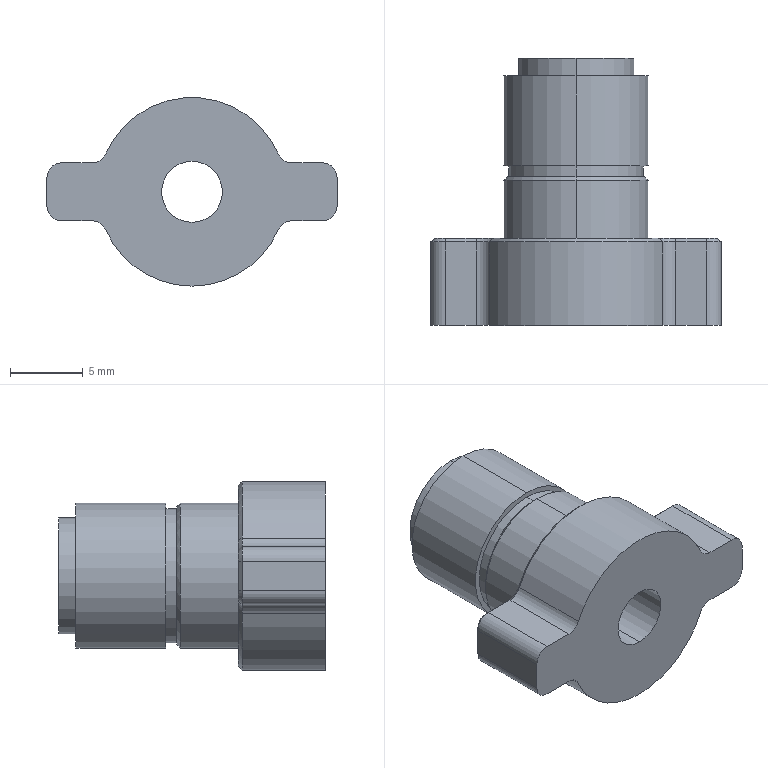Part | SolidWorks | features ICE 5, Chamfer 1, Extrusion 1, HoleWzd 1 | 1 solid | 57 faces | box 20 x 18.4 x 13 mm | volume 1567 mm3 | cylinder 23 | plane 19 | cone 15 | commonest cylinder face diameters 2 x8 10 x4 13 x3 4.2 x2 6 x2 8 x2
STEP:
#1=CARTESIAN_POINT('',(0.,18.15,-3.));
#2=VERTEX_POINT('',#1);
#3=CARTESIAN_POINT('',(0.,18.15,3.));
#4=VERTEX_POINT('',#3);
#5=CARTESIAN_POINT('',(0.,18.15,0.));
#6=DIRECTION('',(0.,1.,0.));
#7=DIRECTION('',(0.,0.,1.));
#8=AXIS2_PLACEMENT_3D('',#5,#6,#7);
#9=CIRCLE('',#8,3.);
#10=EDGE_CURVE('',#2,#4,#9,.T.);
#11=ORIENTED_EDGE('',*,*,#10,.F.);
#12=CARTESIAN_POINT('',(0.,18.4,-3.25));
#13=VERTEX_POINT('',#12);
#14=CARTESIAN_POINT('',(0.,18.15,-3.));
#15=DIRECTION('',(0.,0.7071,-0.7071));
#16=VECTOR('',#15,1000.);
#17=LINE('',#14,#16);
#18=EDGE_CURVE('',#2,#13,#17,.T.);
#19=ORIENTED_EDGE('',*,*,#18,.T.);
#20=CARTESIAN_POINT('',(0.,18.4,3.25));
#21=VERTEX_POINT('',#20);
#22=CARTESIAN_POINT('',(0.,18.4,0.));
#23=DIRECTION('',(0.,-1.,0.));
#24=DIRECTION('',(0.,0.,1.));
#25=AXIS2_PLACEMENT_3D('',#22,#23,#24);
#26=CIRCLE('',#25,3.25);
#27=EDGE_CURVE('',#21,#13,#26,.T.);
#28=ORIENTED_EDGE('',*,*,#27,.F.);
#29=CARTESIAN_POINT('',(0.,18.15,3.));
#30=DIRECTION('',(0.,0.7071,0.7071));
#31=VECTOR('',#30,1000.);
#32=LINE('',#29,#31);
#33=EDGE_CURVE('',#4,#21,#32,.T.);
#34=ORIENTED_EDGE('',*,*,#33,.F.);
#35=EDGE_LOOP('',(#11,#19,#28,#34));
#36=FACE_OUTER_BOUND('',#35,.T.);
#37=CARTESIAN_POINT('',(0.,18.15,0.));
#38=DIRECTION('',(0.,1.,0.));
#39=DIRECTION('',(0.,0.,1.));
#40=AXIS2_PLACEMENT_3D('',#37,#38,#39);
#41=CONICAL_SURFACE('',#40,3.,0.7854);
#42=ADVANCED_FACE('',(#36),#41,.F.);
#43=CARTESIAN_POINT('',(0.,10.25,4.75));
#44=VERTEX_POINT('',#43);
#45=CARTESIAN_POINT('',(0.,10.25,-4.75));
#46=VERTEX_POINT('',#45);
#47=CARTESIAN_POINT('',(0.,10.25,0.));
#48=DIRECTION('',(0.,1.,0.));
#49=DIRECTION('',(0.,0.,1.));
#50=AXIS2_PLACEMENT_3D('',#47,#48,#49);
#51=CIRCLE('',#50,4.75);
#52=EDGE_CURVE('',#44,#46,#51,.T.);
#53=ORIENTED_EDGE('',*,*,#52,.F.);
#54=CARTESIAN_POINT('',(0.,10.,5.));
#55=VERTEX_POINT('',#54);
#56=CARTESIAN_POINT('',(0.,10.25,4.75));
#57=DIRECTION('',(0.,-0.7071,0.7071));
#58=VECTOR('',#57,1000.);
#59=LINE('',#56,#58);
#60=EDGE_CURVE('',#44,#55,#59,.T.);
#61=ORIENTED_EDGE('',*,*,#60,.T.);
#62=CARTESIAN_POINT('',(0.,10.,-5.));
#63=VERTEX_POINT('',#62);
#64=CARTESIAN_POINT('',(0.,10.,0.));
#65=DIRECTION('',(0.,-1.,0.));
#66=DIRECTION('',(0.,0.,1.));
#67=AXIS2_PLACEMENT_3D('',#64,#65,#66);
#68=CIRCLE('',#67,5.);
#69=EDGE_CURVE('',#63,#55,#68,.T.);
#70=ORIENTED_EDGE('',*,*,#69,.F.);
#71=CARTESIAN_POINT('',(0.,10.25,-4.75));
#72=DIRECTION('',(0.,-0.7071,-0.7071));
#73=VECTOR('',#72,1000.);
#74=LINE('',#71,#73);
#75=EDGE_CURVE('',#46,#63,#74,.T.);
#76=ORIENTED_EDGE('',*,*,#75,.F.);
#77=EDGE_LOOP('',(#53,#61,#70,#76));
#78=FACE_OUTER_BOUND('',#77,.T.);
#79=CARTESIAN_POINT('',(0.,10.25,0.));
#80=DIRECTION('',(0.,-1.,0.));
#81=DIRECTION('',(0.,0.,-1.));
#82=AXIS2_PLACEMENT_3D('',#79,#80,#81);
#83=CONICAL_SURFACE('',#82,4.75,0.7854);
#84=ADVANCED_FACE('',(#78),#83,.T.);
#85=CARTESIAN_POINT('',(0.,6.,-6.25));
#86=VERTEX_POINT('',#85);
#87=CARTESIAN_POINT('',(-5.728,6.,-2.5));
#88=VERTEX_POINT('',#87);
#89=CARTESIAN_POINT('',(0.,6.,0.));
#90=DIRECTION('',(0.,1.,0.));
#91=DIRECTION('',(0.,0.,-1.));
#92=AXIS2_PLACEMENT_3D('',#89,#90,#91);
#93=CIRCLE('',#92,6.25);
#94=EDGE_CURVE('',#86,#88,#93,.T.);
#95=ORIENTED_EDGE('',*,*,#94,.F.);
#96=CARTESIAN_POINT('',(0.,5.75,-6.5));
#97=VERTEX_POINT('',#96);
#98=CARTESIAN_POINT('',(0.,6.,-6.25));
#99=DIRECTION('',(0.,-0.7071,-0.7071));
#100=VECTOR('',#99,1000.);
#101=LINE('',#98,#100);
#102=EDGE_CURVE('',#86,#97,#101,.T.);
#103=ORIENTED_EDGE('',*,*,#102,.T.);
#104=CARTESIAN_POINT('',(-5.957,5.75,-2.6));
#105=VERTEX_POINT('',#104);
#106=CARTESIAN_POINT('',(0.,5.75,0.));
#107=DIRECTION('',(0.,-1.,0.));
#108=DIRECTION('',(0.,0.,-1.));
#109=AXIS2_PLACEMENT_3D('',#106,#107,#108);
#110=CIRCLE('',#109,6.5);
#111=EDGE_CURVE('',#105,#97,#110,.T.);
#112=ORIENTED_EDGE('',*,*,#111,.F.);
#113=CARTESIAN_POINT('',(-5.728,6.,-2.5));
#114=DIRECTION('',(-0.6481,-0.7071,-0.2828));
#115=VECTOR('',#114,1000.);
#116=LINE('',#113,#115);
#117=EDGE_CURVE('',#88,#105,#116,.T.);
#118=ORIENTED_EDGE('',*,*,#117,.F.);
#119=EDGE_LOOP('',(#95,#103,#112,#118));
#120=FACE_OUTER_BOUND('',#119,.T.);
#121=CARTESIAN_POINT('',(0.,6.,0.));
#122=DIRECTION('',(0.,-1.,0.));
#123=DIRECTION('',(0.,0.,-1.));
#124=AXIS2_PLACEMENT_3D('',#121,#122,#123);
#125=CONICAL_SURFACE('',#124,6.25,0.7854);
#126=ADVANCED_FACE('',(#120),#125,.T.);
#127=CARTESIAN_POINT('',(0.,13.4,-2.1));
#128=VERTEX_POINT('',#127);
#129=CARTESIAN_POINT('',(0.,13.4,2.1));
#130=VERTEX_POINT('',#129);
#131=CARTESIAN_POINT('',(0.,13.4,0.));
#132=DIRECTION('',(0.,1.,0.));
#133=DIRECTION('',(0.,0.,1.));
#134=AXIS2_PLACEMENT_3D('',#131,#132,#133);
#135=CIRCLE('',#134,2.1);
#136=EDGE_CURVE('',#128,#130,#135,.T.);
#137=ORIENTED_EDGE('',*,*,#136,.T.);
#138=CARTESIAN_POINT('',(0.,0.,2.1));
#139=VERTEX_POINT('',#138);
#140=CARTESIAN_POINT('',(0.,0.,2.1));
#141=DIRECTION('',(0.,-1.,0.));
#142=VECTOR('',#141,1000.);
#143=LINE('',#140,#142);
#144=EDGE_CURVE('',#130,#139,#143,.T.);
#145=ORIENTED_EDGE('',*,*,#144,.T.);
#146=CARTESIAN_POINT('',(0.,0.,-2.1));
#147=VERTEX_POINT('',#146);
#148=CARTESIAN_POINT('',(0.,0.,0.));
#149=DIRECTION('',(0.,-1.,0.));
#150=DIRECTION('',(0.,0.,-1.));
#151=AXIS2_PLACEMENT_3D('',#148,#149,#150);
#152=CIRCLE('',#151,2.1);
#153=EDGE_CURVE('',#139,#147,#152,.T.);
#154=ORIENTED_EDGE('',*,*,#153,.T.);
#155=CARTESIAN_POINT('',(0.,0.,-2.1));
#156=DIRECTION('',(0.,-1.,0.));
#157=VECTOR('',#156,1000.);
#158=LINE('',#155,#157);
#159=EDGE_CURVE('',#128,#147,#158,.T.);
#160=ORIENTED_EDGE('',*,*,#159,.F.);
#161=EDGE_LOOP('',(#137,#145,#154,#160));
#162=FACE_OUTER_BOUND('',#161,.T.);
#163=CARTESIAN_POINT('',(0.,0.,0.));
#164=DIRECTION('',(0.,-1.,0.));
#165=DIRECTION('',(0.,0.,-1.));
#166=AXIS2_PLACEMENT_3D('',#163,#164,#165);
#167=CYLINDRICAL_SURFACE('',#166,2.1);
#168=ADVANCED_FACE('',(#162),#167,.F.);
#169=CARTESIAN_POINT('',(0.,13.4,-3.));
#170=VERTEX_POINT('',#169);
#171=CARTESIAN_POINT('',(0.,13.4,3.));
#172=VERTEX_POINT('',#171);
#173=CARTESIAN_POINT('',(0.,13.4,0.));
#174=DIRECTION('',(0.,1.,0.));
#175=DIRECTION('',(0.,0.,1.));
#176=AXIS2_PLACEMENT_3D('',#173,#174,#175);
#177=CIRCLE('',#176,3.);
#178=EDGE_CURVE('',#170,#172,#177,.T.);
#179=ORIENTED_EDGE('',*,*,#178,.F.);
#180=CARTESIAN_POINT('',(0.,13.4,-3.));
#181=DIRECTION('',(0.,1.,0.));
#182=VECTOR('',#181,1000.);
#183=LINE('',#180,#182);
#184=EDGE_CURVE('',#170,#2,#183,.T.);
#185=ORIENTED_EDGE('',*,*,#184,.T.);
#186=ORIENTED_EDGE('',*,*,#10,.T.);
#187=CARTESIAN_POINT('',(0.,13.4,3.));
#188=DIRECTION('',(0.,1.,0.));
#189=VECTOR('',#188,1000.);
#190=LINE('',#187,#189);
#191=EDGE_CURVE('',#172,#4,#190,.T.);
#192=ORIENTED_EDGE('',*,*,#191,.F.);
#193=EDGE_LOOP('',(#179,#185,#186,#192));
#194=FACE_OUTER_BOUND('',#193,.T.);
#195=CARTESIAN_POINT('',(0.,13.4,0.));
#196=DIRECTION('',(0.,1.,0.));
#197=DIRECTION('',(0.,0.,1.));
#198=AXIS2_PLACEMENT_3D('',#195,#196,#197);
#199=CYLINDRICAL_SURFACE('',#198,3.);
#200=ADVANCED_FACE('',(#194),#199,.F.);
#201=CARTESIAN_POINT('',(0.,18.4,4.));
#202=VERTEX_POINT('',#201);
#203=CARTESIAN_POINT('',(0.,18.4,-4.));
#204=VERTEX_POINT('',#203);
#205=CARTESIAN_POINT('',(0.,18.4,0.));
#206=DIRECTION('',(0.,1.,0.));
#207=DIRECTION('',(0.,0.,1.));
#208=AXIS2_PLACEMENT_3D('',#205,#206,#207);
#209=CIRCLE('',#208,4.);
#210=EDGE_CURVE('',#202,#204,#209,.T.);
#211=ORIENTED_EDGE('',*,*,#210,.F.);
#212=CARTESIAN_POINT('',(0.,17.2,4.));
#213=VERTEX_POINT('',#212);
#214=CARTESIAN_POINT('',(0.,18.4,4.));
#215=DIRECTION('',(0.,-1.,0.));
#216=VECTOR('',#215,1000.);
#217=LINE('',#214,#216);
#218=EDGE_CURVE('',#202,#213,#217,.T.);
#219=ORIENTED_EDGE('',*,*,#218,.T.);
#220=CARTESIAN_POINT('',(0.,17.2,-4.));
#221=VERTEX_POINT('',#220);
#222=CARTESIAN_POINT('',(0.,17.2,0.));
#223=DIRECTION('',(0.,1.,0.));
#224=DIRECTION('',(0.,0.,1.));
#225=AXIS2_PLACEMENT_3D('',#222,#223,#224);
#226=CIRCLE('',#225,4.);
#227=EDGE_CURVE('',#213,#221,#226,.T.);
#228=ORIENTED_EDGE('',*,*,#227,.T.);
#229=CARTESIAN_POINT('',(0.,18.4,-4.));
#230=DIRECTION('',(0.,-1.,0.));
#231=VECTOR('',#230,1000.);
#232=LINE('',#229,#231);
#233=EDGE_CURVE('',#204,#221,#232,.T.);
#234=ORIENTED_EDGE('',*,*,#233,.F.);
#235=EDGE_LOOP('',(#211,#219,#228,#234));
#236=FACE_OUTER_BOUND('',#235,.T.);
#237=CARTESIAN_POINT('',(0.,18.4,0.));
#238=DIRECTION('',(0.,-1.,0.));
#239=DIRECTION('',(0.,0.,-1.));
#240=AXIS2_PLACEMENT_3D('',#237,#238,#239);
#241=CYLINDRICAL_SURFACE('',#240,4.);
#242=ADVANCED_FACE('',(#236),#241,.T.);
#243=CARTESIAN_POINT('',(0.,17.2,5.));
#244=VERTEX_POINT('',#243);
#245=CARTESIAN_POINT('',(0.,17.2,-5.));
#246=VERTEX_POINT('',#245);
#247=CARTESIAN_POINT('',(0.,17.2,0.));
#248=DIRECTION('',(0.,1.,0.));
#249=DIRECTION('',(0.,0.,1.));
#250=AXIS2_PLACEMENT_3D('',#247,#248,#249);
#251=CIRCLE('',#250,5.);
#252=EDGE_CURVE('',#244,#246,#251,.T.);
#253=ORIENTED_EDGE('',*,*,#252,.F.);
#254=CARTESIAN_POINT('',(0.,11.,5.));
#255=VERTEX_POINT('',#254);
#256=CARTESIAN_POINT('',(0.,17.2,5.));
#257=DIRECTION('',(0.,-1.,0.));
#258=VECTOR('',#257,1000.);
#259=LINE('',#256,#258);
#260=EDGE_CURVE('',#244,#255,#259,.T.);
#261=ORIENTED_EDGE('',*,*,#260,.T.);
#262=CARTESIAN_POINT('',(0.,11.,-5.));
#263=VERTEX_POINT('',#262);
#264=CARTESIAN_POINT('',(0.,11.,0.));
#265=DIRECTION('',(0.,1.,0.));
#266=DIRECTION('',(0.,0.,1.));
#267=AXIS2_PLACEMENT_3D('',#264,#265,#266);
#268=CIRCLE('',#267,5.);
#269=EDGE_CURVE('',#255,#263,#268,.T.);
#270=ORIENTED_EDGE('',*,*,#269,.T.);
#271=CARTESIAN_POINT('',(0.,17.2,-5.));
#272=DIRECTION('',(0.,-1.,0.));
#273=VECTOR('',#272,1000.);
#274=LINE('',#271,#273);
#275=EDGE_CURVE('',#246,#263,#274,.T.);
#276=ORIENTED_EDGE('',*,*,#275,.F.);
#277=EDGE_LOOP('',(#253,#261,#270,#276));
#278=FACE_OUTER_BOUND('',#277,.T.);
#279=CARTESIAN_POINT('',(0.,17.2,0.));
#280=DIRECTION('',(0.,-1.,0.));
#281=DIRECTION('',(0.,0.,-1.));
#282=AXIS2_PLACEMENT_3D('',#279,#280,#281);
#283=CYLINDRICAL_SURFACE('',#282,5.);
#284=ADVANCED_FACE('',(#278),#283,.T.);
#285=CARTESIAN_POINT('',(0.,11.,4.625));
#286=VERTEX_POINT('',#285);
#287=CARTESIAN_POINT('',(0.,11.,-4.625));
#288=VERTEX_POINT('',#287);
#289=CARTESIAN_POINT('',(0.,11.,0.));
#290=DIRECTION('',(0.,1.,0.));
#291=DIRECTION('',(0.,0.,1.));
#292=AXIS2_PLACEMENT_3D('',#289,#290,#291);
#293=CIRCLE('',#292,4.625);
#294=EDGE_CURVE('',#286,#288,#293,.T.);
#295=ORIENTED_EDGE('',*,*,#294,.F.);
#296=CARTESIAN_POINT('',(0.,10.25,4.625));
#297=VERTEX_POINT('',#296);
#298=CARTESIAN_POINT('',(0.,11.,4.625));
#299=DIRECTION('',(0.,-1.,0.));
#300=VECTOR('',#299,1000.);
#301=LINE('',#298,#300);
#302=EDGE_CURVE('',#286,#297,#301,.T.);
#303=ORIENTED_EDGE('',*,*,#302,.T.);
#304=CARTESIAN_POINT('',(0.,10.25,-4.625));
#305=VERTEX_POINT('',#304);
#306=CARTESIAN_POINT('',(0.,10.25,0.));
#307=DIRECTION('',(0.,1.,0.));
#308=DIRECTION('',(0.,0.,1.));
#309=AXIS2_PLACEMENT_3D('',#306,#307,#308);
#310=CIRCLE('',#309,4.625);
#311=EDGE_CURVE('',#297,#305,#310,.T.);
#312=ORIENTED_EDGE('',*,*,#311,.T.);
#313=CARTESIAN_POINT('',(0.,11.,-4.625));
#314=DIRECTION('',(0.,-1.,0.));
#315=VECTOR('',#314,1000.);
#316=LINE('',#313,#315);
#317=EDGE_CURVE('',#288,#305,#316,.T.);
#318=ORIENTED_EDGE('',*,*,#317,.F.);
#319=EDGE_LOOP('',(#295,#303,#312,#318));
#320=FACE_OUTER_BOUND('',#319,.T.);
#321=CARTESIAN_POINT('',(0.,11.,0.));
#322=DIRECTION('',(0.,-1.,0.));
#323=DIRECTION('',(0.,0.,-1.));
#324=AXIS2_PLACEMENT_3D('',#321,#322,#323);
#325=CYLINDRICAL_SURFACE('',#324,4.625);
#326=ADVANCED_FACE('',(#320),#325,.T.);
#327=ORIENTED_EDGE('',*,*,#69,.T.);
#328=CARTESIAN_POINT('',(0.,6.,5.));
#329=VERTEX_POINT('',#328);
#330=CARTESIAN_POINT('',(0.,10.25,5.));
#331=DIRECTION('',(0.,-1.,0.));
#332=VECTOR('',#331,1000.);
#333=LINE('',#330,#332);
#334=EDGE_CURVE('',#55,#329,#333,.T.);
#335=ORIENTED_EDGE('',*,*,#334,.T.);
#336=CARTESIAN_POINT('',(0.,6.,-5.));
#337=VERTEX_POINT('',#336);
#338=CARTESIAN_POINT('',(0.,6.,0.));
#339=DIRECTION('',(0.,1.,0.));
#340=DIRECTION('',(0.,0.,1.));
#341=AXIS2_PLACEMENT_3D('',#338,#339,#340);
#342=CIRCLE('',#341,5.);
#343=EDGE_CURVE('',#329,#337,#342,.T.);
#344=ORIENTED_EDGE('',*,*,#343,.T.);
#345=CARTESIAN_POINT('',(0.,10.25,-5.));
#346=DIRECTION('',(0.,-1.,0.));
#347=VECTOR('',#346,1000.);
#348=LINE('',#345,#347);
#349=EDGE_CURVE('',#63,#337,#348,.T.);
#350=ORIENTED_EDGE('',*,*,#349,.F.);
#351=EDGE_LOOP('',(#327,#335,#344,#350));
#352=FACE_OUTER_BOUND('',#351,.T.);
#353=CARTESIAN_POINT('',(0.,10.25,0.));
#354=DIRECTION('',(0.,-1.,0.));
#355=DIRECTION('',(0.,0.,-1.));
#356=AXIS2_PLACEMENT_3D('',#353,#354,#355);
#357=CYLINDRICAL_SURFACE('',#356,5.);
#358=ADVANCED_FACE('',(#352),#357,.T.);
#359=ORIENTED_EDGE('',*,*,#111,.T.);
#360=CARTESIAN_POINT('',(0.,0.,-6.5));
#361=VERTEX_POINT('',#360);
#362=CARTESIAN_POINT('',(0.,6.,-6.5));
#363=DIRECTION('',(0.,-1.,0.));
#364=VECTOR('',#363,1000.);
#365=LINE('',#362,#364);
#366=EDGE_CURVE('',#97,#361,#365,.T.);
#367=ORIENTED_EDGE('',*,*,#366,.T.);
#368=CARTESIAN_POINT('',(-5.957,0.,-2.6));
#369=VERTEX_POINT('',#368);
#370=CARTESIAN_POINT('',(0.,0.,0.));
#371=DIRECTION('',(0.,1.,0.));
#372=DIRECTION('',(0.,0.,1.));
#373=AXIS2_PLACEMENT_3D('',#370,#371,#372);
#374=CIRCLE('',#373,6.5);
#375=EDGE_CURVE('',#361,#369,#374,.T.);
#376=ORIENTED_EDGE('',*,*,#375,.T.);
#377=CARTESIAN_POINT('',(-5.957,6.,-2.6));
#378=DIRECTION('',(0.,-1.,0.));
#379=VECTOR('',#378,1000.);
#380=LINE('',#377,#379);
#381=EDGE_CURVE('',#105,#369,#380,.T.);
#382=ORIENTED_EDGE('',*,*,#381,.F.);
#383=EDGE_LOOP('',(#359,#367,#376,#382));
#384=FACE_OUTER_BOUND('',#383,.T.);
#385=CARTESIAN_POINT('',(0.,6.,0.));
#386=DIRECTION('',(0.,-1.,0.));
#387=DIRECTION('',(0.,0.,-1.));
#388=AXIS2_PLACEMENT_3D('',#385,#386,#387);
#389=CYLINDRICAL_SURFACE('',#388,6.5);
#390=ADVANCED_FACE('',(#384),#389,.T.);
#391=CARTESIAN_POINT('',(5.957,5.75,-2.6));
#392=VERTEX_POINT('',#391);
#393=CARTESIAN_POINT('',(5.957,0.,-2.6));
#394=VERTEX_POINT('',#393);
#395=CARTESIAN_POINT('',(5.957,6.,-2.6));
#396=DIRECTION('',(0.,-1.,0.));
#397=VECTOR('',#396,1000.);
#398=LINE('',#395,#397);
#399=EDGE_CURVE('',#392,#394,#398,.T.);
#400=ORIENTED_EDGE('',*,*,#399,.F.);
#401=CARTESIAN_POINT('',(6.874,5.75,-2.));
#402=VERTEX_POINT('',#401);
#403=CARTESIAN_POINT('',(6.874,5.75,-3.));
#404=DIRECTION('',(0.,1.,0.));
#405=DIRECTION('',(0.,0.,-1.));
#406=AXIS2_PLACEMENT_3D('',#403,#404,#405);
#407=CIRCLE('',#406,1.);
#408=EDGE_CURVE('',#392,#402,#407,.T.);
#409=ORIENTED_EDGE('',*,*,#408,.T.);
#410=CARTESIAN_POINT('',(6.874,0.,-2.));
#411=VERTEX_POINT('',#410);
#412=CARTESIAN_POINT('',(6.874,6.,-2.));
#413=DIRECTION('',(0.,-1.,0.));
#414=VECTOR('',#413,1000.);
#415=LINE('',#412,#414);
#416=EDGE_CURVE('',#402,#411,#415,.T.);
#417=ORIENTED_EDGE('',*,*,#416,.T.);
#418=CARTESIAN_POINT('',(6.874,0.,-3.));
#419=DIRECTION('',(0.,-1.,0.));
#420=DIRECTION('',(0.,0.,-1.));
#421=AXIS2_PLACEMENT_3D('',#418,#419,#420);
#422=CIRCLE('',#421,1.);
#423=EDGE_CURVE('',#411,#394,#422,.T.);
#424=ORIENTED_EDGE('',*,*,#423,.T.);
#425=EDGE_LOOP('',(#400,#409,#417,#424));
#426=FACE_OUTER_BOUND('',#425,.T.);
#427=CARTESIAN_POINT('',(6.874,6.,-3.));
#428=DIRECTION('',(0.,-1.,0.));
#429=DIRECTION('',(0.,0.,-1.));
#430=AXIS2_PLACEMENT_3D('',#427,#428,#429);
#431=CYLINDRICAL_SURFACE('',#430,1.);
#432=ADVANCED_FACE('',(#426),#431,.F.);
#433=ORIENTED_EDGE('',*,*,#366,.F.);
#434=CARTESIAN_POINT('',(0.,5.75,0.));
#435=DIRECTION('',(0.,-1.,0.));
#436=DIRECTION('',(0.,0.,-1.));
#437=AXIS2_PLACEMENT_3D('',#434,#435,#436);
#438=CIRCLE('',#437,6.5);
#439=EDGE_CURVE('',#97,#392,#438,.T.);
#440=ORIENTED_EDGE('',*,*,#439,.T.);
#441=ORIENTED_EDGE('',*,*,#399,.T.);
#442=CARTESIAN_POINT('',(0.,0.,0.));
#443=DIRECTION('',(0.,1.,0.));
#444=DIRECTION('',(0.,0.,1.));
#445=AXIS2_PLACEMENT_3D('',#442,#443,#444);
#446=CIRCLE('',#445,6.5);
#447=EDGE_CURVE('',#394,#361,#446,.T.);
#448=ORIENTED_EDGE('',*,*,#447,.T.);
#449=EDGE_LOOP('',(#433,#440,#441,#448));
#450=FACE_OUTER_BOUND('',#449,.T.);
#451=CARTESIAN_POINT('',(0.,6.,0.));
#452=DIRECTION('',(0.,-1.,0.));
#453=DIRECTION('',(0.,0.,-1.));
#454=AXIS2_PLACEMENT_3D('',#451,#452,#453);
#455=CYLINDRICAL_SURFACE('',#454,6.5);
#456=ADVANCED_FACE('',(#450),#455,.T.);
#457=CARTESIAN_POINT('',(-6.874,5.75,-2.));
#458=VERTEX_POINT('',#457);
#459=CARTESIAN_POINT('',(-6.874,0.,-2.));
#460=VERTEX_POINT('',#459);
#461=CARTESIAN_POINT('',(-6.874,6.,-2.));
#462=DIRECTION('',(0.,-1.,0.));
#463=VECTOR('',#462,1000.);
#464=LINE('',#461,#463);
#465=EDGE_CURVE('',#458,#460,#464,.T.);
#466=ORIENTED_EDGE('',*,*,#465,.F.);
#467=CARTESIAN_POINT('',(-6.874,5.75,-3.));
#468=DIRECTION('',(0.,1.,0.));
#469=DIRECTION('',(0.,0.,-1.));
#470=AXIS2_PLACEMENT_3D('',#467,#468,#469);
#471=CIRCLE('',#470,1.);
#472=EDGE_CURVE('',#458,#105,#471,.T.);
#473=ORIENTED_EDGE('',*,*,#472,.T.);
#474=ORIENTED_EDGE('',*,*,#381,.T.);
#475=CARTESIAN_POINT('',(-6.874,0.,-3.));
#476=DIRECTION('',(0.,-1.,0.));
#477=DIRECTION('',(0.,0.,1.));
#478=AXIS2_PLACEMENT_3D('',#475,#476,#477);
#479=CIRCLE('',#478,1.);
#480=EDGE_CURVE('',#369,#460,#479,.T.);
#481=ORIENTED_EDGE('',*,*,#480,.T.);
#482=EDGE_LOOP('',(#466,#473,#474,#481));
#483=FACE_OUTER_BOUND('',#482,.T.);
#484=CARTESIAN_POINT('',(-6.874,6.,-3.));
#485=DIRECTION('',(0.,-1.,0.));
#486=DIRECTION('',(0.,0.,-1.));
#487=AXIS2_PLACEMENT_3D('',#484,#485,#486);
#488=CYLINDRICAL_SURFACE('',#487,1.);
#489=ADVANCED_FACE('',(#483),#488,.F.);
#490=CARTESIAN_POINT('',(-9.,5.75,-2.));
#491=VERTEX_POINT('',#490);
#492=CARTESIAN_POINT('',(-9.,0.,-2.));
#493=VERTEX_POINT('',#492);
#494=CARTESIAN_POINT('',(-9.,6.,-2.));
#495=DIRECTION('',(0.,-1.,0.));
#496=VECTOR('',#495,1000.);
#497=LINE('',#494,#496);
#498=EDGE_CURVE('',#491,#493,#497,.T.);
#499=ORIENTED_EDGE('',*,*,#498,.F.);
#500=CARTESIAN_POINT('',(-6.874,5.75,-2.));
#501=DIRECTION('',(1.,0.,0.));
#502=VECTOR('',#501,1000.);
#503=LINE('',#500,#502);
#504=EDGE_CURVE('',#491,#458,#503,.T.);
#505=ORIENTED_EDGE('',*,*,#504,.T.);
#506=ORIENTED_EDGE('',*,*,#465,.T.);
#507=CARTESIAN_POINT('',(-6.874,0.,-2.));
#508=DIRECTION('',(-1.,0.,0.));
#509=VECTOR('',#508,1000.);
#510=LINE('',#507,#509);
#511=EDGE_CURVE('',#460,#493,#510,.T.);
#512=ORIENTED_EDGE('',*,*,#511,.T.);
#513=EDGE_LOOP('',(#499,#505,#506,#512));
#514=FACE_OUTER_BOUND('',#513,.T.);
#515=CARTESIAN_POINT('',(-6.874,6.,-2.));
#516=DIRECTION('',(0.,0.,1.));
#517=DIRECTION('',(1.,0.,0.));
#518=AXIS2_PLACEMENT_3D('',#515,#516,#517);
#519=PLANE('',#518);
#520=ADVANCED_FACE('',(#514),#519,.F.);
#521=CARTESIAN_POINT('',(-10.,5.75,-1.));
#522=VERTEX_POINT('',#521);
#523=CARTESIAN_POINT('',(-10.,0.,-1.));
#524=VERTEX_POINT('',#523);
#525=CARTESIAN_POINT('',(-10.,6.,-1.));
#526=DIRECTION('',(0.,-1.,0.));
#527=VECTOR('',#526,1000.);
#528=LINE('',#525,#527);
#529=EDGE_CURVE('',#522,#524,#528,.T.);
#530=ORIENTED_EDGE('',*,*,#529,.F.);
#531=CARTESIAN_POINT('',(-9.,5.75,-1.));
#532=DIRECTION('',(0.,-1.,0.));
#533=DIRECTION('',(0.,0.,-1.));
#534=AXIS2_PLACEMENT_3D('',#531,#532,#533);
#535=CIRCLE('',#534,1.);
#536=EDGE_CURVE('',#522,#491,#535,.T.);
#537=ORIENTED_EDGE('',*,*,#536,.T.);
#538=ORIENTED_EDGE('',*,*,#498,.T.);
#539=CARTESIAN_POINT('',(-9.,0.,-1.));
#540=DIRECTION('',(0.,1.,0.));
#541=DIRECTION('',(0.,0.,1.));
#542=AXIS2_PLACEMENT_3D('',#539,#540,#541);
#543=CIRCLE('',#542,1.);
#544=EDGE_CURVE('',#493,#524,#543,.T.);
#545=ORIENTED_EDGE('',*,*,#544,.T.);
#546=EDGE_LOOP('',(#530,#537,#538,#545));
#547=FACE_OUTER_BOUND('',#546,.T.);
#548=CARTESIAN_POINT('',(-9.,6.,-1.));
#549=DIRECTION('',(0.,-1.,0.));
#550=DIRECTION('',(0.,0.,-1.));
#551=AXIS2_PLACEMENT_3D('',#548,#549,#550);
#552=CYLINDRICAL_SURFACE('',#551,1.);
#553=ADVANCED_FACE('',(#547),#552,.T.);
#554=CARTESIAN_POINT('',(-10.,5.75,1.));
#555=VERTEX_POINT('',#554);
#556=CARTESIAN_POINT('',(-10.,0.,1.));
#557=VERTEX_POINT('',#556);
#558=CARTESIAN_POINT('',(-10.,6.,1.));
#559=DIRECTION('',(0.,-1.,0.));
#560=VECTOR('',#559,1000.);
#561=LINE('',#558,#560);
#562=EDGE_CURVE('',#555,#557,#561,.T.);
#563=ORIENTED_EDGE('',*,*,#562,.F.);
#564=CARTESIAN_POINT('',(-10.,5.75,-1.));
#565=DIRECTION('',(0.,0.,-1.));
#566=VECTOR('',#565,1000.);
#567=LINE('',#564,#566);
#568=EDGE_CURVE('',#555,#522,#567,.T.);
#569=ORIENTED_EDGE('',*,*,#568,.T.);
#570=ORIENTED_EDGE('',*,*,#529,.T.);
#571=CARTESIAN_POINT('',(-10.,0.,-1.));
#572=DIRECTION('',(0.,0.,1.));
#573=VECTOR('',#572,1000.);
#574=LINE('',#571,#573);
#575=EDGE_CURVE('',#524,#557,#574,.T.);
#576=ORIENTED_EDGE('',*,*,#575,.T.);
#577=EDGE_LOOP('',(#563,#569,#570,#576));
#578=FACE_OUTER_BOUND('',#577,.T.);
#579=CARTESIAN_POINT('',(-10.,6.,-1.));
#580=DIRECTION('',(1.,0.,0.));
#581=DIRECTION('',(0.,0.,-1.));
#582=AXIS2_PLACEMENT_3D('',#579,#580,#581);
#583=PLANE('',#582);
#584=ADVANCED_FACE('',(#578),#583,.F.);
#585=CARTESIAN_POINT('',(-9.,5.75,2.));
#586=VERTEX_POINT('',#585);
#587=CARTESIAN_POINT('',(-9.,0.,2.));
#588=VERTEX_POINT('',#587);
#589=CARTESIAN_POINT('',(-9.,6.,2.));
#590=DIRECTION('',(0.,-1.,0.));
#591=VECTOR('',#590,1000.);
#592=LINE('',#589,#591);
#593=EDGE_CURVE('',#586,#588,#592,.T.);
#594=ORIENTED_EDGE('',*,*,#593,.F.);
#595=CARTESIAN_POINT('',(-9.,5.75,1.));
#596=DIRECTION('',(0.,-1.,0.));
#597=DIRECTION('',(0.,0.,-1.));
#598=AXIS2_PLACEMENT_3D('',#595,#596,#597);
#599=CIRCLE('',#598,1.);
#600=EDGE_CURVE('',#586,#555,#599,.T.);
#601=ORIENTED_EDGE('',*,*,#600,.T.);
#602=ORIENTED_EDGE('',*,*,#562,.T.);
#603=CARTESIAN_POINT('',(-9.,0.,1.));
#604=DIRECTION('',(0.,1.,0.));
#605=DIRECTION('',(0.,0.,1.));
#606=AXIS2_PLACEMENT_3D('',#603,#604,#605);
#607=CIRCLE('',#606,1.);
#608=EDGE_CURVE('',#557,#588,#607,.T.);
#609=ORIENTED_EDGE('',*,*,#608,.T.);
#610=EDGE_LOOP('',(#594,#601,#602,#609));
#611=FACE_OUTER_BOUND('',#610,.T.);
#612=CARTESIAN_POINT('',(-9.,6.,1.));
#613=DIRECTION('',(0.,-1.,0.));
#614=DIRECTION('',(0.,0.,-1.));
#615=AXIS2_PLACEMENT_3D('',#612,#613,#614);
#616=CYLINDRICAL_SURFACE('',#615,1.);
#617=ADVANCED_FACE('',(#611),#616,.T.);
#618=CARTESIAN_POINT('',(-6.874,5.75,2.));
#619=VERTEX_POINT('',#618);
#620=CARTESIAN_POINT('',(-6.874,0.,2.));
#621=VERTEX_POINT('',#620);
#622=CARTESIAN_POINT('',(-6.874,6.,2.));
#623=DIRECTION('',(0.,-1.,0.));
#624=VECTOR('',#623,1000.);
#625=LINE('',#622,#624);
#626=EDGE_CURVE('',#619,#621,#625,.T.);
#627=ORIENTED_EDGE('',*,*,#626,.F.);
#628=CARTESIAN_POINT('',(-9.,5.75,2.));
#629=DIRECTION('',(-1.,0.,0.));
#630=VECTOR('',#629,1000.);
#631=LINE('',#628,#630);
#632=EDGE_CURVE('',#619,#586,#631,.T.);
#633=ORIENTED_EDGE('',*,*,#632,.T.);
#634=ORIENTED_EDGE('',*,*,#593,.T.);
#635=CARTESIAN_POINT('',(-9.,0.,2.));
#636=DIRECTION('',(1.,0.,0.));
#637=VECTOR('',#636,1000.);
#638=LINE('',#635,#637);
#639=EDGE_CURVE('',#588,#621,#638,.T.);
#640=ORIENTED_EDGE('',*,*,#639,.T.);
#641=EDGE_LOOP('',(#627,#633,#634,#640));
#642=FACE_OUTER_BOUND('',#641,.T.);
#643=CARTESIAN_POINT('',(-9.,6.,2.));
#644=DIRECTION('',(0.,0.,-1.));
#645=DIRECTION('',(-1.,0.,0.));
#646=AXIS2_PLACEMENT_3D('',#643,#644,#645);
#647=PLANE('',#646);
#648=ADVANCED_FACE('',(#642),#647,.F.);
#649=CARTESIAN_POINT('',(-5.957,5.75,2.6));
#650=VERTEX_POINT('',#649);
#651=CARTESIAN_POINT('',(-5.957,0.,2.6));
#652=VERTEX_POINT('',#651);
#653=CARTESIAN_POINT('',(-5.957,6.,2.6));
#654=DIRECTION('',(0.,-1.,0.));
#655=VECTOR('',#654,1000.);
#656=LINE('',#653,#655);
#657=EDGE_CURVE('',#650,#652,#656,.T.);
#658=ORIENTED_EDGE('',*,*,#657,.F.);
#659=CARTESIAN_POINT('',(-6.874,5.75,3.));
#660=DIRECTION('',(0.,1.,0.));
#661=DIRECTION('',(0.,0.,-1.));
#662=AXIS2_PLACEMENT_3D('',#659,#660,#661);
#663=CIRCLE('',#662,1.);
#664=EDGE_CURVE('',#650,#619,#663,.T.);
#665=ORIENTED_EDGE('',*,*,#664,.T.);
#666=ORIENTED_EDGE('',*,*,#626,.T.);
#667=CARTESIAN_POINT('',(-6.874,0.,3.));
#668=DIRECTION('',(0.,-1.,0.));
#669=DIRECTION('',(0.,0.,-1.));
#670=AXIS2_PLACEMENT_3D('',#667,#668,#669);
#671=CIRCLE('',#670,1.);
#672=EDGE_CURVE('',#621,#652,#671,.T.);
#673=ORIENTED_EDGE('',*,*,#672,.T.);
#674=EDGE_LOOP('',(#658,#665,#666,#673));
#675=FACE_OUTER_BOUND('',#674,.T.);
#676=CARTESIAN_POINT('',(-6.874,6.,3.));
#677=DIRECTION('',(0.,-1.,0.));
#678=DIRECTION('',(0.,0.,-1.));
#679=AXIS2_PLACEMENT_3D('',#676,#677,#678);
#680=CYLINDRICAL_SURFACE('',#679,1.);
#681=ADVANCED_FACE('',(#675),#680,.F.);
#682=CARTESIAN_POINT('',(5.957,5.75,2.6));
#683=VERTEX_POINT('',#682);
#684=CARTESIAN_POINT('',(5.957,0.,2.6));
#685=VERTEX_POINT('',#684);
#686=CARTESIAN_POINT('',(5.957,6.,2.6));
#687=DIRECTION('',(0.,-1.,0.));
#688=VECTOR('',#687,1000.);
#689=LINE('',#686,#688);
#690=EDGE_CURVE('',#683,#685,#689,.T.);
#691=ORIENTED_EDGE('',*,*,#690,.F.);
#692=CARTESIAN_POINT('',(0.,5.75,0.));
#693=DIRECTION('',(0.,-1.,0.));
#694=DIRECTION('',(0.,0.,-1.));
#695=AXIS2_PLACEMENT_3D('',#692,#693,#694);
#696=CIRCLE('',#695,6.5);
#697=EDGE_CURVE('',#683,#650,#696,.T.);
#698=ORIENTED_EDGE('',*,*,#697,.T.);
#699=ORIENTED_EDGE('',*,*,#657,.T.);
#700=CARTESIAN_POINT('',(0.,0.,0.));
#701=DIRECTION('',(0.,1.,0.));
#702=DIRECTION('',(0.,0.,1.));
#703=AXIS2_PLACEMENT_3D('',#700,#701,#702);
#704=CIRCLE('',#703,6.5);
#705=EDGE_CURVE('',#652,#685,#704,.T.);
#706=ORIENTED_EDGE('',*,*,#705,.T.);
#707=EDGE_LOOP('',(#691,#698,#699,#706));
#708=FACE_OUTER_BOUND('',#707,.T.);
#709=CARTESIAN_POINT('',(0.,6.,0.));
#710=DIRECTION('',(0.,-1.,0.));
#711=DIRECTION('',(0.,0.,-1.));
#712=AXIS2_PLACEMENT_3D('',#709,#710,#711);
#713=CYLINDRICAL_SURFACE('',#712,6.5);
#714=ADVANCED_FACE('',(#708),#713,.T.);
#715=CARTESIAN_POINT('',(6.874,5.75,2.));
#716=VERTEX_POINT('',#715);
#717=CARTESIAN_POINT('',(6.874,0.,2.));
#718=VERTEX_POINT('',#717);
#719=CARTESIAN_POINT('',(6.874,6.,2.));
#720=DIRECTION('',(0.,-1.,0.));
#721=VECTOR('',#720,1000.);
#722=LINE('',#719,#721);
#723=EDGE_CURVE('',#716,#718,#722,.T.);
#724=ORIENTED_EDGE('',*,*,#723,.F.);
#725=CARTESIAN_POINT('',(6.874,5.75,3.));
#726=DIRECTION('',(0.,1.,0.));
#727=DIRECTION('',(0.,0.,-1.));
#728=AXIS2_PLACEMENT_3D('',#725,#726,#727);
#729=CIRCLE('',#728,1.);
#730=EDGE_CURVE('',#716,#683,#729,.T.);
#731=ORIENTED_EDGE('',*,*,#730,.T.);
#732=ORIENTED_EDGE('',*,*,#690,.T.);
#733=CARTESIAN_POINT('',(6.874,0.,3.));
#734=DIRECTION('',(0.,-1.,0.));
#735=DIRECTION('',(0.,0.,1.));
#736=AXIS2_PLACEMENT_3D('',#733,#734,#735);
#737=CIRCLE('',#736,1.);
#738=EDGE_CURVE('',#685,#718,#737,.T.);
#739=ORIENTED_EDGE('',*,*,#738,.T.);
#740=EDGE_LOOP('',(#724,#731,#732,#739));
#741=FACE_OUTER_BOUND('',#740,.T.);
#742=CARTESIAN_POINT('',(6.874,6.,3.));
#743=DIRECTION('',(0.,-1.,0.));
#744=DIRECTION('',(0.,0.,-1.));
#745=AXIS2_PLACEMENT_3D('',#742,#743,#744);
#746=CYLINDRICAL_SURFACE('',#745,1.);
#747=ADVANCED_FACE('',(#741),#746,.F.);
#748=CARTESIAN_POINT('',(9.,5.75,2.));
#749=VERTEX_POINT('',#748);
#750=CARTESIAN_POINT('',(9.,0.,2.));
#751=VERTEX_POINT('',#750);
#752=CARTESIAN_POINT('',(9.,6.,2.));
#753=DIRECTION('',(0.,-1.,0.));
#754=VECTOR('',#753,1000.);
#755=LINE('',#752,#754);
#756=EDGE_CURVE('',#749,#751,#755,.T.);
#757=ORIENTED_EDGE('',*,*,#756,.F.);
#758=CARTESIAN_POINT('',(9.,5.75,2.));
#759=DIRECTION('',(-1.,0.,0.));
#760=VECTOR('',#759,1000.);
#761=LINE('',#758,#760);
#762=EDGE_CURVE('',#749,#716,#761,.T.);
#763=ORIENTED_EDGE('',*,*,#762,.T.);
#764=ORIENTED_EDGE('',*,*,#723,.T.);
#765=CARTESIAN_POINT('',(9.,0.,2.));
#766=DIRECTION('',(1.,0.,0.));
#767=VECTOR('',#766,1000.);
#768=LINE('',#765,#767);
#769=EDGE_CURVE('',#718,#751,#768,.T.);
#770=ORIENTED_EDGE('',*,*,#769,.T.);
#771=EDGE_LOOP('',(#757,#763,#764,#770));
#772=FACE_OUTER_BOUND('',#771,.T.);
#773=CARTESIAN_POINT('',(9.,6.,2.));
#774=DIRECTION('',(0.,0.,-1.));
#775=DIRECTION('',(-1.,0.,0.));
#776=AXIS2_PLACEMENT_3D('',#773,#774,#775);
#777=PLANE('',#776);
#778=ADVANCED_FACE('',(#772),#777,.F.);
#779=CARTESIAN_POINT('',(10.,5.75,1.));
#780=VERTEX_POINT('',#779);
#781=CARTESIAN_POINT('',(10.,0.,1.));
#782=VERTEX_POINT('',#781);
#783=CARTESIAN_POINT('',(10.,6.,1.));
#784=DIRECTION('',(0.,-1.,0.));
#785=VECTOR('',#784,1000.);
#786=LINE('',#783,#785);
#787=EDGE_CURVE('',#780,#782,#786,.T.);
#788=ORIENTED_EDGE('',*,*,#787,.F.);
#789=CARTESIAN_POINT('',(9.,5.75,1.));
#790=DIRECTION('',(0.,-1.,0.));
#791=DIRECTION('',(0.,0.,-1.));
#792=AXIS2_PLACEMENT_3D('',#789,#790,#791);
#793=CIRCLE('',#792,1.);
#794=EDGE_CURVE('',#780,#749,#793,.T.);
#795=ORIENTED_EDGE('',*,*,#794,.T.);
#796=ORIENTED_EDGE('',*,*,#756,.T.);
#797=CARTESIAN_POINT('',(9.,0.,1.));
#798=DIRECTION('',(0.,1.,0.));
#799=DIRECTION('',(0.,0.,-1.));
#800=AXIS2_PLACEMENT_3D('',#797,#798,#799);
#801=CIRCLE('',#800,1.);
#802=EDGE_CURVE('',#751,#782,#801,.T.);
#803=ORIENTED_EDGE('',*,*,#802,.T.);
#804=EDGE_LOOP('',(#788,#795,#796,#803));
#805=FACE_OUTER_BOUND('',#804,.T.);
#806=CARTESIAN_POINT('',(9.,6.,1.));
#807=DIRECTION('',(0.,-1.,0.));
#808=DIRECTION('',(0.,0.,-1.));
#809=AXIS2_PLACEMENT_3D('',#806,#807,#808);
#810=CYLINDRICAL_SURFACE('',#809,1.);
#811=ADVANCED_FACE('',(#805),#810,.T.);
#812=CARTESIAN_POINT('',(10.,5.75,-1.));
#813=VERTEX_POINT('',#812);
#814=CARTESIAN_POINT('',(10.,0.,-1.));
#815=VERTEX_POINT('',#814);
#816=CARTESIAN_POINT('',(10.,6.,-1.));
#817=DIRECTION('',(0.,-1.,0.));
#818=VECTOR('',#817,1000.);
#819=LINE('',#816,#818);
#820=EDGE_CURVE('',#813,#815,#819,.T.);
#821=ORIENTED_EDGE('',*,*,#820,.F.);
#822=CARTESIAN_POINT('',(10.,5.75,-1.));
#823=DIRECTION('',(0.,0.,1.));
#824=VECTOR('',#823,1000.);
#825=LINE('',#822,#824);
#826=EDGE_CURVE('',#813,#780,#825,.T.);
#827=ORIENTED_EDGE('',*,*,#826,.T.);
#828=ORIENTED_EDGE('',*,*,#787,.T.);
#829=CARTESIAN_POINT('',(10.,0.,-1.));
#830=DIRECTION('',(0.,0.,-1.));
#831=VECTOR('',#830,1000.);
#832=LINE('',#829,#831);
#833=EDGE_CURVE('',#782,#815,#832,.T.);
#834=ORIENTED_EDGE('',*,*,#833,.T.);
#835=EDGE_LOOP('',(#821,#827,#828,#834));
#836=FACE_OUTER_BOUND('',#835,.T.);
#837=CARTESIAN_POINT('',(10.,6.,-1.));
#838=DIRECTION('',(-1.,0.,0.));
#839=DIRECTION('',(0.,0.,1.));
#840=AXIS2_PLACEMENT_3D('',#837,#838,#839);
#841=PLANE('',#840);
#842=ADVANCED_FACE('',(#836),#841,.F.);
#843=CARTESIAN_POINT('',(9.,5.75,-2.));
#844=VERTEX_POINT('',#843);
#845=CARTESIAN_POINT('',(9.,0.,-2.));
#846=VERTEX_POINT('',#845);
#847=CARTESIAN_POINT('',(9.,6.,-2.));
#848=DIRECTION('',(0.,-1.,0.));
#849=VECTOR('',#848,1000.);
#850=LINE('',#847,#849);
#851=EDGE_CURVE('',#844,#846,#850,.T.);
#852=ORIENTED_EDGE('',*,*,#851,.F.);
#853=CARTESIAN_POINT('',(9.,5.75,-1.));
#854=DIRECTION('',(0.,-1.,0.));
#855=DIRECTION('',(0.,0.,-1.));
#856=AXIS2_PLACEMENT_3D('',#853,#854,#855);
#857=CIRCLE('',#856,1.);
#858=EDGE_CURVE('',#844,#813,#857,.T.);
#859=ORIENTED_EDGE('',*,*,#858,.T.);
#860=ORIENTED_EDGE('',*,*,#820,.T.);
#861=CARTESIAN_POINT('',(9.,0.,-1.));
#862=DIRECTION('',(0.,1.,0.));
#863=DIRECTION('',(0.,0.,-1.));
#864=AXIS2_PLACEMENT_3D('',#861,#862,#863);
#865=CIRCLE('',#864,1.);
#866=EDGE_CURVE('',#815,#846,#865,.T.);
#867=ORIENTED_EDGE('',*,*,#866,.T.);
#868=EDGE_LOOP('',(#852,#859,#860,#867));
#869=FACE_OUTER_BOUND('',#868,.T.);
#870=CARTESIAN_POINT('',(9.,6.,-1.));
#871=DIRECTION('',(0.,-1.,0.));
#872=DIRECTION('',(0.,0.,-1.));
#873=AXIS2_PLACEMENT_3D('',#870,#871,#872);
#874=CYLINDRICAL_SURFACE('',#873,1.);
#875=ADVANCED_FACE('',(#869),#874,.T.);
#876=ORIENTED_EDGE('',*,*,#416,.F.);
#877=CARTESIAN_POINT('',(6.874,5.75,-2.));
#878=DIRECTION('',(1.,0.,0.));
#879=VECTOR('',#878,1000.);
#880=LINE('',#877,#879);
#881=EDGE_CURVE('',#402,#844,#880,.T.);
#882=ORIENTED_EDGE('',*,*,#881,.T.);
#883=ORIENTED_EDGE('',*,*,#851,.T.);
#884=CARTESIAN_POINT('',(6.874,0.,-2.));
#885=DIRECTION('',(-1.,0.,0.));
#886=VECTOR('',#885,1000.);
#887=LINE('',#884,#886);
#888=EDGE_CURVE('',#846,#411,#887,.T.);
#889=ORIENTED_EDGE('',*,*,#888,.T.);
#890=EDGE_LOOP('',(#876,#882,#883,#889));
#891=FACE_OUTER_BOUND('',#890,.T.);
#892=CARTESIAN_POINT('',(6.874,6.,-2.));
#893=DIRECTION('',(0.,0.,1.));
#894=DIRECTION('',(1.,0.,0.));
#895=AXIS2_PLACEMENT_3D('',#892,#893,#894);
#896=PLANE('',#895);
#897=ADVANCED_FACE('',(#891),#896,.F.);
#898=CARTESIAN_POINT('',(-6.874,6.,1.75));
#899=VERTEX_POINT('',#898);
#900=CARTESIAN_POINT('',(-5.728,6.,2.5));
#901=VERTEX_POINT('',#900);
#902=CARTESIAN_POINT('',(-6.874,6.,3.));
#903=DIRECTION('',(0.,-1.,0.));
#904=DIRECTION('',(0.,0.,-1.));
#905=AXIS2_PLACEMENT_3D('',#902,#903,#904);
#906=CIRCLE('',#905,1.25);
#907=EDGE_CURVE('',#899,#901,#906,.T.);
#908=ORIENTED_EDGE('',*,*,#907,.T.);
#909=CARTESIAN_POINT('',(5.728,6.,2.5));
#910=VERTEX_POINT('',#909);
#911=CARTESIAN_POINT('',(0.,6.,0.));
#912=DIRECTION('',(0.,1.,0.));
#913=DIRECTION('',(0.,0.,-1.));
#914=AXIS2_PLACEMENT_3D('',#911,#912,#913);
#915=CIRCLE('',#914,6.25);
#916=EDGE_CURVE('',#901,#910,#915,.T.);
#917=ORIENTED_EDGE('',*,*,#916,.T.);
#918=CARTESIAN_POINT('',(6.874,6.,1.75));
#919=VERTEX_POINT('',#918);
#920=CARTESIAN_POINT('',(6.874,6.,3.));
#921=DIRECTION('',(0.,-1.,0.));
#922=DIRECTION('',(0.,0.,-1.));
#923=AXIS2_PLACEMENT_3D('',#920,#921,#922);
#924=CIRCLE('',#923,1.25);
#925=EDGE_CURVE('',#910,#919,#924,.T.);
#926=ORIENTED_EDGE('',*,*,#925,.T.);
#927=CARTESIAN_POINT('',(9.,6.,1.75));
#928=VERTEX_POINT('',#927);
#929=CARTESIAN_POINT('',(6.874,6.,1.75));
#930=DIRECTION('',(1.,0.,0.));
#931=VECTOR('',#930,1000.);
#932=LINE('',#929,#931);
#933=EDGE_CURVE('',#919,#928,#932,.T.);
#934=ORIENTED_EDGE('',*,*,#933,.T.);
#935=CARTESIAN_POINT('',(9.75,6.,1.));
#936=VERTEX_POINT('',#935);
#937=CARTESIAN_POINT('',(9.,6.,1.));
#938=DIRECTION('',(0.,1.,0.));
#939=DIRECTION('',(0.,0.,-1.));
#940=AXIS2_PLACEMENT_3D('',#937,#938,#939);
#941=CIRCLE('',#940,0.75);
#942=EDGE_CURVE('',#928,#936,#941,.T.);
#943=ORIENTED_EDGE('',*,*,#942,.T.);
#944=CARTESIAN_POINT('',(9.75,6.,-1.));
#945=VERTEX_POINT('',#944);
#946=CARTESIAN_POINT('',(9.75,6.,-3.));
#947=DIRECTION('',(0.,0.,-1.));
#948=VECTOR('',#947,1000.);
#949=LINE('',#946,#948);
#950=EDGE_CURVE('',#936,#945,#949,.T.);
#951=ORIENTED_EDGE('',*,*,#950,.T.);
#952=CARTESIAN_POINT('',(9.,6.,-1.75));
#953=VERTEX_POINT('',#952);
#954=CARTESIAN_POINT('',(9.,6.,-1.));
#955=DIRECTION('',(0.,1.,0.));
#956=DIRECTION('',(0.,0.,-1.));
#957=AXIS2_PLACEMENT_3D('',#954,#955,#956);
#958=CIRCLE('',#957,0.75);
#959=EDGE_CURVE('',#945,#953,#958,.T.);
#960=ORIENTED_EDGE('',*,*,#959,.T.);
#961=CARTESIAN_POINT('',(6.874,6.,-1.75));
#962=VERTEX_POINT('',#961);
#963=CARTESIAN_POINT('',(6.874,6.,-1.75));
#964=DIRECTION('',(-1.,0.,0.));
#965=VECTOR('',#964,1000.);
#966=LINE('',#963,#965);
#967=EDGE_CURVE('',#953,#962,#966,.T.);
#968=ORIENTED_EDGE('',*,*,#967,.T.);
#969=CARTESIAN_POINT('',(5.728,6.,-2.5));
#970=VERTEX_POINT('',#969);
#971=CARTESIAN_POINT('',(6.874,6.,-3.));
#972=DIRECTION('',(0.,-1.,0.));
#973=DIRECTION('',(0.,0.,-1.));
#974=AXIS2_PLACEMENT_3D('',#971,#972,#973);
#975=CIRCLE('',#974,1.25);
#976=EDGE_CURVE('',#962,#970,#975,.T.);
#977=ORIENTED_EDGE('',*,*,#976,.T.);
#978=CARTESIAN_POINT('',(0.,6.,0.));
#979=DIRECTION('',(0.,1.,0.));
#980=DIRECTION('',(0.,0.,-1.));
#981=AXIS2_PLACEMENT_3D('',#978,#979,#980);
#982=CIRCLE('',#981,6.25);
#983=EDGE_CURVE('',#970,#86,#982,.T.);
#984=ORIENTED_EDGE('',*,*,#983,.T.);
#985=ORIENTED_EDGE('',*,*,#94,.T.);
#986=CARTESIAN_POINT('',(-6.874,6.,-1.75));
#987=VERTEX_POINT('',#986);
#988=CARTESIAN_POINT('',(-6.874,6.,-3.));
#989=DIRECTION('',(0.,-1.,0.));
#990=DIRECTION('',(0.,0.,-1.));
#991=AXIS2_PLACEMENT_3D('',#988,#989,#990);
#992=CIRCLE('',#991,1.25);
#993=EDGE_CURVE('',#88,#987,#992,.T.);
#994=ORIENTED_EDGE('',*,*,#993,.T.);
#995=CARTESIAN_POINT('',(-9.,6.,-1.75));
#996=VERTEX_POINT('',#995);
#997=CARTESIAN_POINT('',(6.874,6.,-1.75));
#998=DIRECTION('',(-1.,0.,0.));
#999=VECTOR('',#998,1000.);
#1000=LINE('',#997,#999);
#1001=EDGE_CURVE('',#987,#996,#1000,.T.);
#1002=ORIENTED_EDGE('',*,*,#1001,.T.);
#1003=CARTESIAN_POINT('',(-9.75,6.,-1.));
#1004=VERTEX_POINT('',#1003);
#1005=CARTESIAN_POINT('',(-9.,6.,-1.));
#1006=DIRECTION('',(0.,1.,0.));
#1007=DIRECTION('',(0.,0.,-1.));
#1008=AXIS2_PLACEMENT_3D('',#1005,#1006,#1007);
#1009=CIRCLE('',#1008,0.75);
#1010=EDGE_CURVE('',#996,#1004,#1009,.T.);
#1011=ORIENTED_EDGE('',*,*,#1010,.T.);
#1012=CARTESIAN_POINT('',(-9.75,6.,1.));
#1013=VERTEX_POINT('',#1012);
#1014=CARTESIAN_POINT('',(-9.75,6.,-3.));
#1015=DIRECTION('',(0.,0.,1.));
#1016=VECTOR('',#1015,1000.);
#1017=LINE('',#1014,#1016);
#1018=EDGE_CURVE('',#1004,#1013,#1017,.T.);
#1019=ORIENTED_EDGE('',*,*,#1018,.T.);
#1020=CARTESIAN_POINT('',(-9.,6.,1.75));
#1021=VERTEX_POINT('',#1020);
#1022=CARTESIAN_POINT('',(-9.,6.,1.));
#1023=DIRECTION('',(0.,1.,0.));
#1024=DIRECTION('',(0.,0.,-1.));
#1025=AXIS2_PLACEMENT_3D('',#1022,#1023,#1024);
#1026=CIRCLE('',#1025,0.75);
#1027=EDGE_CURVE('',#1013,#1021,#1026,.T.);
#1028=ORIENTED_EDGE('',*,*,#1027,.T.);
#1029=CARTESIAN_POINT('',(6.874,6.,1.75));
#1030=DIRECTION('',(1.,0.,0.));
#1031=VECTOR('',#1030,1000.);
#1032=LINE('',#1029,#1031);
#1033=EDGE_CURVE('',#1021,#899,#1032,.T.);
#1034=ORIENTED_EDGE('',*,*,#1033,.T.);
#1035=EDGE_LOOP('',(#908,#917,#926,#934,#943,#951,#960,#968,#977,#984,#985,#994,#1002,#1011,#1019,#1028,#1034));
#1036=FACE_OUTER_BOUND('',#1035,.T.);
#1037=CARTESIAN_POINT('',(0.,6.,0.));
#1038=DIRECTION('',(0.,1.,0.));
#1039=DIRECTION('',(0.,0.,1.));
#1040=AXIS2_PLACEMENT_3D('',#1037,#1038,#1039);
#1041=CIRCLE('',#1040,5.);
#1042=EDGE_CURVE('',#337,#329,#1041,.T.);
#1043=ORIENTED_EDGE('',*,*,#1042,.F.);
#1044=ORIENTED_EDGE('',*,*,#343,.F.);
#1045=EDGE_LOOP('',(#1043,#1044));
#1046=FACE_BOUND('',#1045,.T.);
#1047=CARTESIAN_POINT('',(6.874,6.,-3.));
#1048=DIRECTION('',(0.,-1.,0.));
#1049=DIRECTION('',(0.,0.,-1.));
#1050=AXIS2_PLACEMENT_3D('',#1047,#1048,#1049);
#1051=PLANE('',#1050);
#1052=ADVANCED_FACE('',(#1036,#1046),#1051,.F.);
#1053=CARTESIAN_POINT('',(0.,0.,0.));
#1054=DIRECTION('',(0.,-1.,0.));
#1055=DIRECTION('',(0.,0.,-1.));
#1056=AXIS2_PLACEMENT_3D('',#1053,#1054,#1055);
#1057=CIRCLE('',#1056,2.1);
#1058=EDGE_CURVE('',#147,#139,#1057,.T.);
#1059=ORIENTED_EDGE('',*,*,#1058,.F.);
#1060=ORIENTED_EDGE('',*,*,#153,.F.);
#1061=EDGE_LOOP('',(#1059,#1060));
#1062=FACE_BOUND('',#1061,.T.);
#1063=ORIENTED_EDGE('',*,*,#423,.F.);
#1064=ORIENTED_EDGE('',*,*,#888,.F.);
#1065=ORIENTED_EDGE('',*,*,#866,.F.);
#1066=ORIENTED_EDGE('',*,*,#833,.F.);
#1067=ORIENTED_EDGE('',*,*,#802,.F.);
#1068=ORIENTED_EDGE('',*,*,#769,.F.);
#1069=ORIENTED_EDGE('',*,*,#738,.F.);
#1070=ORIENTED_EDGE('',*,*,#705,.F.);
#1071=ORIENTED_EDGE('',*,*,#672,.F.);
#1072=ORIENTED_EDGE('',*,*,#639,.F.);
#1073=ORIENTED_EDGE('',*,*,#608,.F.);
#1074=ORIENTED_EDGE('',*,*,#575,.F.);
#1075=ORIENTED_EDGE('',*,*,#544,.F.);
#1076=ORIENTED_EDGE('',*,*,#511,.F.);
#1077=ORIENTED_EDGE('',*,*,#480,.F.);
#1078=ORIENTED_EDGE('',*,*,#375,.F.);
#1079=ORIENTED_EDGE('',*,*,#447,.F.);
#1080=EDGE_LOOP('',(#1063,#1064,#1065,#1066,#1067,#1068,#1069,#1070,#1071,#1072,#1073,#1074,#1075,#1076,#1077,#1078,#1079));
#1081=FACE_OUTER_BOUND('',#1080,.T.);
#1082=CARTESIAN_POINT('',(6.874,0.,-3.));
#1083=DIRECTION('',(0.,-1.,0.));
#1084=DIRECTION('',(0.,0.,-1.));
#1085=AXIS2_PLACEMENT_3D('',#1082,#1083,#1084);
#1086=PLANE('',#1085);
#1087=ADVANCED_FACE('',(#1062,#1081),#1086,.T.);
#1088=ORIENTED_EDGE('',*,*,#334,.F.);
#1089=CARTESIAN_POINT('',(0.,10.,0.));
#1090=DIRECTION('',(0.,-1.,0.));
#1091=DIRECTION('',(0.,0.,1.));
#1092=AXIS2_PLACEMENT_3D('',#1089,#1090,#1091);
#1093=CIRCLE('',#1092,5.);
#1094=EDGE_CURVE('',#55,#63,#1093,.T.);
#1095=ORIENTED_EDGE('',*,*,#1094,.T.);
#1096=ORIENTED_EDGE('',*,*,#349,.T.);
#1097=ORIENTED_EDGE('',*,*,#1042,.T.);
#1098=EDGE_LOOP('',(#1088,#1095,#1096,#1097));
#1099=FACE_OUTER_BOUND('',#1098,.T.);
#1100=CARTESIAN_POINT('',(0.,10.25,0.));
#1101=DIRECTION('',(0.,-1.,0.));
#1102=DIRECTION('',(0.,0.,-1.));
#1103=AXIS2_PLACEMENT_3D('',#1100,#1101,#1102);
#1104=CYLINDRICAL_SURFACE('',#1103,5.);
#1105=ADVANCED_FACE('',(#1099),#1104,.T.);
#1106=CARTESIAN_POINT('',(0.,10.25,0.));
#1107=DIRECTION('',(0.,1.,0.));
#1108=DIRECTION('',(0.,0.,1.));
#1109=AXIS2_PLACEMENT_3D('',#1106,#1107,#1108);
#1110=CIRCLE('',#1109,4.75);
#1111=EDGE_CURVE('',#46,#44,#1110,.T.);
#1112=ORIENTED_EDGE('',*,*,#1111,.T.);
#1113=ORIENTED_EDGE('',*,*,#52,.T.);
#1114=EDGE_LOOP('',(#1112,#1113));
#1115=FACE_OUTER_BOUND('',#1114,.T.);
#1116=CARTESIAN_POINT('',(0.,10.25,0.));
#1117=DIRECTION('',(0.,1.,0.));
#1118=DIRECTION('',(0.,0.,1.));
#1119=AXIS2_PLACEMENT_3D('',#1116,#1117,#1118);
#1120=CIRCLE('',#1119,4.625);
#1121=EDGE_CURVE('',#305,#297,#1120,.T.);
#1122=ORIENTED_EDGE('',*,*,#1121,.F.);
#1123=ORIENTED_EDGE('',*,*,#311,.F.);
#1124=EDGE_LOOP('',(#1122,#1123));
#1125=FACE_BOUND('',#1124,.T.);
#1126=CARTESIAN_POINT('',(0.,10.25,0.));
#1127=DIRECTION('',(0.,1.,0.));
#1128=DIRECTION('',(0.,0.,1.));
#1129=AXIS2_PLACEMENT_3D('',#1126,#1127,#1128);
#1130=PLANE('',#1129);
#1131=ADVANCED_FACE('',(#1115,#1125),#1130,.T.);
#1132=ORIENTED_EDGE('',*,*,#302,.F.);
#1133=CARTESIAN_POINT('',(0.,11.,0.));
#1134=DIRECTION('',(0.,1.,0.));
#1135=DIRECTION('',(0.,0.,1.));
#1136=AXIS2_PLACEMENT_3D('',#1133,#1134,#1135);
#1137=CIRCLE('',#1136,4.625);
#1138=EDGE_CURVE('',#288,#286,#1137,.T.);
#1139=ORIENTED_EDGE('',*,*,#1138,.F.);
#1140=ORIENTED_EDGE('',*,*,#317,.T.);
#1141=ORIENTED_EDGE('',*,*,#1121,.T.);
#1142=EDGE_LOOP('',(#1132,#1139,#1140,#1141));
#1143=FACE_OUTER_BOUND('',#1142,.T.);
#1144=CARTESIAN_POINT('',(0.,11.,0.));
#1145=DIRECTION('',(0.,-1.,0.));
#1146=DIRECTION('',(0.,0.,-1.));
#1147=AXIS2_PLACEMENT_3D('',#1144,#1145,#1146);
#1148=CYLINDRICAL_SURFACE('',#1147,4.625);
#1149=ADVANCED_FACE('',(#1143),#1148,.T.);
#1150=ORIENTED_EDGE('',*,*,#260,.F.);
#1151=CARTESIAN_POINT('',(0.,17.2,0.));
#1152=DIRECTION('',(0.,1.,0.));
#1153=DIRECTION('',(0.,0.,1.));
#1154=AXIS2_PLACEMENT_3D('',#1151,#1152,#1153);
#1155=CIRCLE('',#1154,5.);
#1156=EDGE_CURVE('',#246,#244,#1155,.T.);
#1157=ORIENTED_EDGE('',*,*,#1156,.F.);
#1158=ORIENTED_EDGE('',*,*,#275,.T.);
#1159=CARTESIAN_POINT('',(0.,11.,0.));
#1160=DIRECTION('',(0.,1.,0.));
#1161=DIRECTION('',(0.,0.,1.));
#1162=AXIS2_PLACEMENT_3D('',#1159,#1160,#1161);
#1163=CIRCLE('',#1162,5.);
#1164=EDGE_CURVE('',#263,#255,#1163,.T.);
#1165=ORIENTED_EDGE('',*,*,#1164,.T.);
#1166=EDGE_LOOP('',(#1150,#1157,#1158,#1165));
#1167=FACE_OUTER_BOUND('',#1166,.T.);
#1168=CARTESIAN_POINT('',(0.,17.2,0.));
#1169=DIRECTION('',(0.,-1.,0.));
#1170=DIRECTION('',(0.,0.,-1.));
#1171=AXIS2_PLACEMENT_3D('',#1168,#1169,#1170);
#1172=CYLINDRICAL_SURFACE('',#1171,5.);
#1173=ADVANCED_FACE('',(#1167),#1172,.T.);
#1174=CARTESIAN_POINT('',(0.,17.2,0.));
#1175=DIRECTION('',(0.,1.,0.));
#1176=DIRECTION('',(0.,0.,1.));
#1177=AXIS2_PLACEMENT_3D('',#1174,#1175,#1176);
#1178=CIRCLE('',#1177,4.);
#1179=EDGE_CURVE('',#221,#213,#1178,.T.);
#1180=ORIENTED_EDGE('',*,*,#1179,.F.);
#1181=ORIENTED_EDGE('',*,*,#227,.F.);
#1182=EDGE_LOOP('',(#1180,#1181));
#1183=FACE_BOUND('',#1182,.T.);
#1184=ORIENTED_EDGE('',*,*,#1156,.T.);
#1185=ORIENTED_EDGE('',*,*,#252,.T.);
#1186=EDGE_LOOP('',(#1184,#1185));
#1187=FACE_OUTER_BOUND('',#1186,.T.);
#1188=CARTESIAN_POINT('',(0.,17.2,0.));
#1189=DIRECTION('',(0.,1.,0.));
#1190=DIRECTION('',(0.,0.,1.));
#1191=AXIS2_PLACEMENT_3D('',#1188,#1189,#1190);
#1192=PLANE('',#1191);
#1193=ADVANCED_FACE('',(#1183,#1187),#1192,.T.);
#1194=ORIENTED_EDGE('',*,*,#1138,.T.);
#1195=ORIENTED_EDGE('',*,*,#294,.T.);
#1196=EDGE_LOOP('',(#1194,#1195));
#1197=FACE_BOUND('',#1196,.T.);
#1198=ORIENTED_EDGE('',*,*,#1164,.F.);
#1199=ORIENTED_EDGE('',*,*,#269,.F.);
#1200=EDGE_LOOP('',(#1198,#1199));
#1201=FACE_OUTER_BOUND('',#1200,.T.);
#1202=CARTESIAN_POINT('',(0.,11.,0.));
#1203=DIRECTION('',(0.,1.,0.));
#1204=DIRECTION('',(0.,0.,1.));
#1205=AXIS2_PLACEMENT_3D('',#1202,#1203,#1204);
#1206=PLANE('',#1205);
#1207=ADVANCED_FACE('',(#1197,#1201),#1206,.F.);
#1208=ORIENTED_EDGE('',*,*,#218,.F.);
#1209=CARTESIAN_POINT('',(0.,18.4,0.));
#1210=DIRECTION('',(0.,1.,0.));
#1211=DIRECTION('',(0.,0.,1.));
#1212=AXIS2_PLACEMENT_3D('',#1209,#1210,#1211);
#1213=CIRCLE('',#1212,4.);
#1214=EDGE_CURVE('',#204,#202,#1213,.T.);
#1215=ORIENTED_EDGE('',*,*,#1214,.F.);
#1216=ORIENTED_EDGE('',*,*,#233,.T.);
#1217=ORIENTED_EDGE('',*,*,#1179,.T.);
#1218=EDGE_LOOP('',(#1208,#1215,#1216,#1217));
#1219=FACE_OUTER_BOUND('',#1218,.T.);
#1220=CARTESIAN_POINT('',(0.,18.4,0.));
#1221=DIRECTION('',(0.,-1.,0.));
#1222=DIRECTION('',(0.,0.,-1.));
#1223=AXIS2_PLACEMENT_3D('',#1220,#1221,#1222);
#1224=CYLINDRICAL_SURFACE('',#1223,4.);
#1225=ADVANCED_FACE('',(#1219),#1224,.T.);
#1226=ORIENTED_EDGE('',*,*,#27,.T.);
#1227=CARTESIAN_POINT('',(0.,18.4,0.));
#1228=DIRECTION('',(0.,-1.,0.));
#1229=DIRECTION('',(0.,0.,1.));
#1230=AXIS2_PLACEMENT_3D('',#1227,#1228,#1229);
#1231=CIRCLE('',#1230,3.25);
#1232=EDGE_CURVE('',#13,#21,#1231,.T.);
#1233=ORIENTED_EDGE('',*,*,#1232,.T.);
#1234=EDGE_LOOP('',(#1226,#1233));
#1235=FACE_BOUND('',#1234,.T.);
#1236=ORIENTED_EDGE('',*,*,#1214,.T.);
#1237=ORIENTED_EDGE('',*,*,#210,.T.);
#1238=EDGE_LOOP('',(#1236,#1237));
#1239=FACE_OUTER_BOUND('',#1238,.T.);
#1240=CARTESIAN_POINT('',(0.,18.4,0.));
#1241=DIRECTION('',(0.,1.,0.));
#1242=DIRECTION('',(0.,0.,1.));
#1243=AXIS2_PLACEMENT_3D('',#1240,#1241,#1242);
#1244=PLANE('',#1243);
#1245=ADVANCED_FACE('',(#1235,#1239),#1244,.T.);
#1246=ORIENTED_EDGE('',*,*,#184,.F.);
#1247=CARTESIAN_POINT('',(0.,13.4,0.));
#1248=DIRECTION('',(0.,1.,0.));
#1249=DIRECTION('',(0.,0.,1.));
#1250=AXIS2_PLACEMENT_3D('',#1247,#1248,#1249);
#1251=CIRCLE('',#1250,3.);
#1252=EDGE_CURVE('',#172,#170,#1251,.T.);
#1253=ORIENTED_EDGE('',*,*,#1252,.F.);
#1254=ORIENTED_EDGE('',*,*,#191,.T.);
#1255=CARTESIAN_POINT('',(0.,18.15,0.));
#1256=DIRECTION('',(0.,1.,0.));
#1257=DIRECTION('',(0.,0.,1.));
#1258=AXIS2_PLACEMENT_3D('',#1255,#1256,#1257);
#1259=CIRCLE('',#1258,3.);
#1260=EDGE_CURVE('',#4,#2,#1259,.T.);
#1261=ORIENTED_EDGE('',*,*,#1260,.T.);
#1262=EDGE_LOOP('',(#1246,#1253,#1254,#1261));
#1263=FACE_OUTER_BOUND('',#1262,.T.);
#1264=CARTESIAN_POINT('',(0.,13.4,0.));
#1265=DIRECTION('',(0.,1.,0.));
#1266=DIRECTION('',(0.,0.,1.));
#1267=AXIS2_PLACEMENT_3D('',#1264,#1265,#1266);
#1268=CYLINDRICAL_SURFACE('',#1267,3.);
#1269=ADVANCED_FACE('',(#1263),#1268,.F.);
#1270=ORIENTED_EDGE('',*,*,#136,.F.);
#1271=CARTESIAN_POINT('',(0.,13.4,0.));
#1272=DIRECTION('',(0.,1.,0.));
#1273=DIRECTION('',(0.,0.,1.));
#1274=AXIS2_PLACEMENT_3D('',#1271,#1272,#1273);
#1275=CIRCLE('',#1274,2.1);
#1276=EDGE_CURVE('',#130,#128,#1275,.T.);
#1277=ORIENTED_EDGE('',*,*,#1276,.F.);
#1278=EDGE_LOOP('',(#1270,#1277));
#1279=FACE_BOUND('',#1278,.T.);
#1280=ORIENTED_EDGE('',*,*,#1252,.T.);
#1281=ORIENTED_EDGE('',*,*,#178,.T.);
#1282=EDGE_LOOP('',(#1280,#1281));
#1283=FACE_OUTER_BOUND('',#1282,.T.);
#1284=CARTESIAN_POINT('',(0.,13.4,0.));
#1285=DIRECTION('',(0.,1.,0.));
#1286=DIRECTION('',(0.,0.,1.));
#1287=AXIS2_PLACEMENT_3D('',#1284,#1285,#1286);
#1288=PLANE('',#1287);
#1289=ADVANCED_FACE('',(#1279,#1283),#1288,.T.);
#1290=ORIENTED_EDGE('',*,*,#144,.F.);
#1291=ORIENTED_EDGE('',*,*,#1276,.T.);
#1292=ORIENTED_EDGE('',*,*,#159,.T.);
#1293=ORIENTED_EDGE('',*,*,#1058,.T.);
#1294=EDGE_LOOP('',(#1290,#1291,#1292,#1293));
#1295=FACE_OUTER_BOUND('',#1294,.T.);
#1296=CARTESIAN_POINT('',(0.,0.,0.));
#1297=DIRECTION('',(0.,-1.,0.));
#1298=DIRECTION('',(0.,0.,-1.));
#1299=AXIS2_PLACEMENT_3D('',#1296,#1297,#1298);
#1300=CYLINDRICAL_SURFACE('',#1299,2.1);
#1301=ADVANCED_FACE('',(#1295),#1300,.F.);
#1302=ORIENTED_EDGE('',*,*,#102,.F.);
#1303=ORIENTED_EDGE('',*,*,#983,.F.);
#1304=CARTESIAN_POINT('',(5.957,5.75,-2.6));
#1305=DIRECTION('',(-0.6481,0.7071,0.2828));
#1306=VECTOR('',#1305,1000.);
#1307=LINE('',#1304,#1306);
#1308=EDGE_CURVE('',#392,#970,#1307,.T.);
#1309=ORIENTED_EDGE('',*,*,#1308,.F.);
#1310=ORIENTED_EDGE('',*,*,#439,.F.);
#1311=EDGE_LOOP('',(#1302,#1303,#1309,#1310));
#1312=FACE_OUTER_BOUND('',#1311,.T.);
#1313=CARTESIAN_POINT('',(0.,6.,0.));
#1314=DIRECTION('',(0.,-1.,0.));
#1315=DIRECTION('',(0.,0.,-1.));
#1316=AXIS2_PLACEMENT_3D('',#1313,#1314,#1315);
#1317=CONICAL_SURFACE('',#1316,6.25,0.7854);
#1318=ADVANCED_FACE('',(#1312),#1317,.T.);
#1319=ORIENTED_EDGE('',*,*,#117,.T.);
#1320=ORIENTED_EDGE('',*,*,#472,.F.);
#1321=CARTESIAN_POINT('',(-6.874,6.,-1.75));
#1322=DIRECTION('',(0.,-0.7071,-0.7071));
#1323=VECTOR('',#1322,1000.);
#1324=LINE('',#1321,#1323);
#1325=EDGE_CURVE('',#987,#458,#1324,.T.);
#1326=ORIENTED_EDGE('',*,*,#1325,.F.);
#1327=ORIENTED_EDGE('',*,*,#993,.F.);
#1328=EDGE_LOOP('',(#1319,#1320,#1326,#1327));
#1329=FACE_OUTER_BOUND('',#1328,.T.);
#1330=CARTESIAN_POINT('',(-6.874,6.,-3.));
#1331=DIRECTION('',(0.,1.,0.));
#1332=DIRECTION('',(0.,0.,1.));
#1333=AXIS2_PLACEMENT_3D('',#1330,#1331,#1332);
#1334=CONICAL_SURFACE('',#1333,1.25,0.7854);
#1335=ADVANCED_FACE('',(#1329),#1334,.F.);
#1336=ORIENTED_EDGE('',*,*,#1308,.T.);
#1337=ORIENTED_EDGE('',*,*,#976,.F.);
#1338=CARTESIAN_POINT('',(6.874,5.75,-2.));
#1339=DIRECTION('',(0.,0.7071,0.7071));
#1340=VECTOR('',#1339,1000.);
#1341=LINE('',#1338,#1340);
#1342=EDGE_CURVE('',#402,#962,#1341,.T.);
#1343=ORIENTED_EDGE('',*,*,#1342,.F.);
#1344=ORIENTED_EDGE('',*,*,#408,.F.);
#1345=EDGE_LOOP('',(#1336,#1337,#1343,#1344));
#1346=FACE_OUTER_BOUND('',#1345,.T.);
#1347=CARTESIAN_POINT('',(6.874,6.,-3.));
#1348=DIRECTION('',(0.,1.,0.));
#1349=DIRECTION('',(0.,0.,1.));
#1350=AXIS2_PLACEMENT_3D('',#1347,#1348,#1349);
#1351=CONICAL_SURFACE('',#1350,1.25,0.7854);
#1352=ADVANCED_FACE('',(#1346),#1351,.F.);
#1353=ORIENTED_EDGE('',*,*,#1325,.T.);
#1354=ORIENTED_EDGE('',*,*,#504,.F.);
#1355=CARTESIAN_POINT('',(-9.,6.,-1.75));
#1356=DIRECTION('',(0.,-0.7071,-0.7071));
#1357=VECTOR('',#1356,1000.);
#1358=LINE('',#1355,#1357);
#1359=EDGE_CURVE('',#996,#491,#1358,.T.);
#1360=ORIENTED_EDGE('',*,*,#1359,.F.);
#1361=ORIENTED_EDGE('',*,*,#1001,.F.);
#1362=EDGE_LOOP('',(#1353,#1354,#1360,#1361));
#1363=FACE_OUTER_BOUND('',#1362,.T.);
#1364=CARTESIAN_POINT('',(6.874,6.,-1.75));
#1365=DIRECTION('',(0.,-0.7071,0.7071));
#1366=DIRECTION('',(-1.,0.,0.));
#1367=AXIS2_PLACEMENT_3D('',#1364,#1365,#1366);
#1368=PLANE('',#1367);
#1369=ADVANCED_FACE('',(#1363),#1368,.F.);
#1370=ORIENTED_EDGE('',*,*,#1342,.T.);
#1371=ORIENTED_EDGE('',*,*,#967,.F.);
#1372=CARTESIAN_POINT('',(9.,5.75,-2.));
#1373=DIRECTION('',(0.,0.7071,0.7071));
#1374=VECTOR('',#1373,1000.);
#1375=LINE('',#1372,#1374);
#1376=EDGE_CURVE('',#844,#953,#1375,.T.);
#1377=ORIENTED_EDGE('',*,*,#1376,.F.);
#1378=ORIENTED_EDGE('',*,*,#881,.F.);
#1379=EDGE_LOOP('',(#1370,#1371,#1377,#1378));
#1380=FACE_OUTER_BOUND('',#1379,.T.);
#1381=CARTESIAN_POINT('',(6.874,6.,-1.75));
#1382=DIRECTION('',(0.,-0.7071,0.7071));
#1383=DIRECTION('',(-1.,0.,0.));
#1384=AXIS2_PLACEMENT_3D('',#1381,#1382,#1383);
#1385=PLANE('',#1384);
#1386=ADVANCED_FACE('',(#1380),#1385,.F.);
#1387=ORIENTED_EDGE('',*,*,#1359,.T.);
#1388=ORIENTED_EDGE('',*,*,#536,.F.);
#1389=CARTESIAN_POINT('',(-9.75,6.,-1.));
#1390=DIRECTION('',(-0.7071,-0.7071,0.));
#1391=VECTOR('',#1390,1000.);
#1392=LINE('',#1389,#1391);
#1393=EDGE_CURVE('',#1004,#522,#1392,.T.);
#1394=ORIENTED_EDGE('',*,*,#1393,.F.);
#1395=ORIENTED_EDGE('',*,*,#1010,.F.);
#1396=EDGE_LOOP('',(#1387,#1388,#1394,#1395));
#1397=FACE_OUTER_BOUND('',#1396,.T.);
#1398=CARTESIAN_POINT('',(-9.,6.,-1.));
#1399=DIRECTION('',(0.,-1.,0.));
#1400=DIRECTION('',(0.,0.,-1.));
#1401=AXIS2_PLACEMENT_3D('',#1398,#1399,#1400);
#1402=CONICAL_SURFACE('',#1401,0.75,0.7854);
#1403=ADVANCED_FACE('',(#1397),#1402,.T.);
#1404=ORIENTED_EDGE('',*,*,#1376,.T.);
#1405=ORIENTED_EDGE('',*,*,#959,.F.);
#1406=CARTESIAN_POINT('',(10.,5.75,-1.));
#1407=DIRECTION('',(-0.7071,0.7071,0.));
#1408=VECTOR('',#1407,1000.);
#1409=LINE('',#1406,#1408);
#1410=EDGE_CURVE('',#813,#945,#1409,.T.);
#1411=ORIENTED_EDGE('',*,*,#1410,.F.);
#1412=ORIENTED_EDGE('',*,*,#858,.F.);
#1413=EDGE_LOOP('',(#1404,#1405,#1411,#1412));
#1414=FACE_OUTER_BOUND('',#1413,.T.);
#1415=CARTESIAN_POINT('',(9.,6.,-1.));
#1416=DIRECTION('',(0.,-1.,0.));
#1417=DIRECTION('',(0.,0.,-1.));
#1418=AXIS2_PLACEMENT_3D('',#1415,#1416,#1417);
#1419=CONICAL_SURFACE('',#1418,0.75,0.7854);
#1420=ADVANCED_FACE('',(#1414),#1419,.T.);
#1421=ORIENTED_EDGE('',*,*,#1393,.T.);
#1422=ORIENTED_EDGE('',*,*,#568,.F.);
#1423=CARTESIAN_POINT('',(-9.75,6.,1.));
#1424=DIRECTION('',(-0.7071,-0.7071,0.));
#1425=VECTOR('',#1424,1000.);
#1426=LINE('',#1423,#1425);
#1427=EDGE_CURVE('',#1013,#555,#1426,.T.);
#1428=ORIENTED_EDGE('',*,*,#1427,.F.);
#1429=ORIENTED_EDGE('',*,*,#1018,.F.);
#1430=EDGE_LOOP('',(#1421,#1422,#1428,#1429));
#1431=FACE_OUTER_BOUND('',#1430,.T.);
#1432=CARTESIAN_POINT('',(-9.75,6.,-3.));
#1433=DIRECTION('',(0.7071,-0.7071,0.));
#1434=DIRECTION('',(0.,0.,1.));
#1435=AXIS2_PLACEMENT_3D('',#1432,#1433,#1434);
#1436=PLANE('',#1435);
#1437=ADVANCED_FACE('',(#1431),#1436,.F.);
#1438=ORIENTED_EDGE('',*,*,#1410,.T.);
#1439=ORIENTED_EDGE('',*,*,#950,.F.);
#1440=CARTESIAN_POINT('',(10.,5.75,1.));
#1441=DIRECTION('',(-0.7071,0.7071,0.));
#1442=VECTOR('',#1441,1000.);
#1443=LINE('',#1440,#1442);
#1444=EDGE_CURVE('',#780,#936,#1443,.T.);
#1445=ORIENTED_EDGE('',*,*,#1444,.F.);
#1446=ORIENTED_EDGE('',*,*,#826,.F.);
#1447=EDGE_LOOP('',(#1438,#1439,#1445,#1446));
#1448=FACE_OUTER_BOUND('',#1447,.T.);
#1449=CARTESIAN_POINT('',(9.75,6.,-3.));
#1450=DIRECTION('',(-0.7071,-0.7071,0.));
#1451=DIRECTION('',(0.,0.,-1.));
#1452=AXIS2_PLACEMENT_3D('',#1449,#1450,#1451);
#1453=PLANE('',#1452);
#1454=ADVANCED_FACE('',(#1448),#1453,.F.);
#1455=ORIENTED_EDGE('',*,*,#1427,.T.);
#1456=ORIENTED_EDGE('',*,*,#600,.F.);
#1457=CARTESIAN_POINT('',(-9.,6.,1.75));
#1458=DIRECTION('',(0.,-0.7071,0.7071));
#1459=VECTOR('',#1458,1000.);
#1460=LINE('',#1457,#1459);
#1461=EDGE_CURVE('',#1021,#586,#1460,.T.);
#1462=ORIENTED_EDGE('',*,*,#1461,.F.);
#1463=ORIENTED_EDGE('',*,*,#1027,.F.);
#1464=EDGE_LOOP('',(#1455,#1456,#1462,#1463));
#1465=FACE_OUTER_BOUND('',#1464,.T.);
#1466=CARTESIAN_POINT('',(-9.,6.,1.));
#1467=DIRECTION('',(0.,-1.,0.));
#1468=DIRECTION('',(0.,0.,-1.));
#1469=AXIS2_PLACEMENT_3D('',#1466,#1467,#1468);
#1470=CONICAL_SURFACE('',#1469,0.75,0.7854);
#1471=ADVANCED_FACE('',(#1465),#1470,.T.);
#1472=ORIENTED_EDGE('',*,*,#1444,.T.);
#1473=ORIENTED_EDGE('',*,*,#942,.F.);
#1474=CARTESIAN_POINT('',(9.,5.75,2.));
#1475=DIRECTION('',(0.,0.7071,-0.7071));
#1476=VECTOR('',#1475,1000.);
#1477=LINE('',#1474,#1476);
#1478=EDGE_CURVE('',#749,#928,#1477,.T.);
#1479=ORIENTED_EDGE('',*,*,#1478,.F.);
#1480=ORIENTED_EDGE('',*,*,#794,.F.);
#1481=EDGE_LOOP('',(#1472,#1473,#1479,#1480));
#1482=FACE_OUTER_BOUND('',#1481,.T.);
#1483=CARTESIAN_POINT('',(9.,6.,1.));
#1484=DIRECTION('',(0.,-1.,0.));
#1485=DIRECTION('',(0.,0.,-1.));
#1486=AXIS2_PLACEMENT_3D('',#1483,#1484,#1485);
#1487=CONICAL_SURFACE('',#1486,0.75,0.7854);
#1488=ADVANCED_FACE('',(#1482),#1487,.T.);
#1489=ORIENTED_EDGE('',*,*,#1461,.T.);
#1490=ORIENTED_EDGE('',*,*,#632,.F.);
#1491=CARTESIAN_POINT('',(-6.874,6.,1.75));
#1492=DIRECTION('',(0.,-0.7071,0.7071));
#1493=VECTOR('',#1492,1000.);
#1494=LINE('',#1491,#1493);
#1495=EDGE_CURVE('',#899,#619,#1494,.T.);
#1496=ORIENTED_EDGE('',*,*,#1495,.F.);
#1497=ORIENTED_EDGE('',*,*,#1033,.F.);
#1498=EDGE_LOOP('',(#1489,#1490,#1496,#1497));
#1499=FACE_OUTER_BOUND('',#1498,.T.);
#1500=CARTESIAN_POINT('',(6.874,6.,1.75));
#1501=DIRECTION('',(0.,-0.7071,-0.7071));
#1502=DIRECTION('',(1.,0.,0.));
#1503=AXIS2_PLACEMENT_3D('',#1500,#1501,#1502);
#1504=PLANE('',#1503);
#1505=ADVANCED_FACE('',(#1499),#1504,.F.);
#1506=ORIENTED_EDGE('',*,*,#1478,.T.);
#1507=ORIENTED_EDGE('',*,*,#933,.F.);
#1508=CARTESIAN_POINT('',(6.874,5.75,2.));
#1509=DIRECTION('',(0.,0.7071,-0.7071));
#1510=VECTOR('',#1509,1000.);
#1511=LINE('',#1508,#1510);
#1512=EDGE_CURVE('',#716,#919,#1511,.T.);
#1513=ORIENTED_EDGE('',*,*,#1512,.F.);
#1514=ORIENTED_EDGE('',*,*,#762,.F.);
#1515=EDGE_LOOP('',(#1506,#1507,#1513,#1514));
#1516=FACE_OUTER_BOUND('',#1515,.T.);
#1517=CARTESIAN_POINT('',(6.874,6.,1.75));
#1518=DIRECTION('',(0.,-0.7071,-0.7071));
#1519=DIRECTION('',(1.,0.,0.));
#1520=AXIS2_PLACEMENT_3D('',#1517,#1518,#1519);
#1521=PLANE('',#1520);
#1522=ADVANCED_FACE('',(#1516),#1521,.F.);
#1523=ORIENTED_EDGE('',*,*,#1495,.T.);
#1524=ORIENTED_EDGE('',*,*,#664,.F.);
#1525=CARTESIAN_POINT('',(-5.728,6.,2.5));
#1526=DIRECTION('',(-0.6481,-0.7071,0.2828));
#1527=VECTOR('',#1526,1000.);
#1528=LINE('',#1525,#1527);
#1529=EDGE_CURVE('',#901,#650,#1528,.T.);
#1530=ORIENTED_EDGE('',*,*,#1529,.F.);
#1531=ORIENTED_EDGE('',*,*,#907,.F.);
#1532=EDGE_LOOP('',(#1523,#1524,#1530,#1531));
#1533=FACE_OUTER_BOUND('',#1532,.T.);
#1534=CARTESIAN_POINT('',(-6.874,6.,3.));
#1535=DIRECTION('',(0.,1.,0.));
#1536=DIRECTION('',(0.,0.,1.));
#1537=AXIS2_PLACEMENT_3D('',#1534,#1535,#1536);
#1538=CONICAL_SURFACE('',#1537,1.25,0.7854);
#1539=ADVANCED_FACE('',(#1533),#1538,.F.);
#1540=ORIENTED_EDGE('',*,*,#1512,.T.);
#1541=ORIENTED_EDGE('',*,*,#925,.F.);
#1542=CARTESIAN_POINT('',(5.957,5.75,2.6));
#1543=DIRECTION('',(-0.6481,0.7071,-0.2828));
#1544=VECTOR('',#1543,1000.);
#1545=LINE('',#1542,#1544);
#1546=EDGE_CURVE('',#683,#910,#1545,.T.);
#1547=ORIENTED_EDGE('',*,*,#1546,.F.);
#1548=ORIENTED_EDGE('',*,*,#730,.F.);
#1549=EDGE_LOOP('',(#1540,#1541,#1547,#1548));
#1550=FACE_OUTER_BOUND('',#1549,.T.);
#1551=CARTESIAN_POINT('',(6.874,6.,3.));
#1552=DIRECTION('',(0.,1.,0.));
#1553=DIRECTION('',(0.,0.,1.));
#1554=AXIS2_PLACEMENT_3D('',#1551,#1552,#1553);
#1555=CONICAL_SURFACE('',#1554,1.25,0.7854);
#1556=ADVANCED_FACE('',(#1550),#1555,.F.);
#1557=ORIENTED_EDGE('',*,*,#1529,.T.);
#1558=ORIENTED_EDGE('',*,*,#697,.F.);
#1559=ORIENTED_EDGE('',*,*,#1546,.T.);
#1560=ORIENTED_EDGE('',*,*,#916,.F.);
#1561=EDGE_LOOP('',(#1557,#1558,#1559,#1560));
#1562=FACE_OUTER_BOUND('',#1561,.T.);
#1563=CARTESIAN_POINT('',(0.,6.,0.));
#1564=DIRECTION('',(0.,-1.,0.));
#1565=DIRECTION('',(0.,0.,-1.));
#1566=AXIS2_PLACEMENT_3D('',#1563,#1564,#1565);
#1567=CONICAL_SURFACE('',#1566,6.25,0.7854);
#1568=ADVANCED_FACE('',(#1562),#1567,.T.);
#1569=ORIENTED_EDGE('',*,*,#60,.F.);
#1570=ORIENTED_EDGE('',*,*,#1111,.F.);
#1571=ORIENTED_EDGE('',*,*,#75,.T.);
#1572=ORIENTED_EDGE('',*,*,#1094,.F.);
#1573=EDGE_LOOP('',(#1569,#1570,#1571,#1572));
#1574=FACE_OUTER_BOUND('',#1573,.T.);
#1575=CARTESIAN_POINT('',(0.,10.25,0.));
#1576=DIRECTION('',(0.,-1.,0.));
#1577=DIRECTION('',(0.,0.,-1.));
#1578=AXIS2_PLACEMENT_3D('',#1575,#1576,#1577);
#1579=CONICAL_SURFACE('',#1578,4.75,0.7854);
#1580=ADVANCED_FACE('',(#1574),#1579,.T.);
#1581=ORIENTED_EDGE('',*,*,#18,.F.);
#1582=ORIENTED_EDGE('',*,*,#1260,.F.);
#1583=ORIENTED_EDGE('',*,*,#33,.T.);
#1584=ORIENTED_EDGE('',*,*,#1232,.F.);
#1585=EDGE_LOOP('',(#1581,#1582,#1583,#1584));
#1586=FACE_OUTER_BOUND('',#1585,.T.);
#1587=CARTESIAN_POINT('',(0.,18.15,0.));
#1588=DIRECTION('',(0.,1.,0.));
#1589=DIRECTION('',(0.,0.,1.));
#1590=AXIS2_PLACEMENT_3D('',#1587,#1588,#1589);
#1591=CONICAL_SURFACE('',#1590,3.,0.7854);
#1592=ADVANCED_FACE('',(#1586),#1591,.F.);
#1593=CLOSED_SHELL('',(#42,#84,#126,#168,#200,#242,#284,#326,#358,#390,#432,#456,#489,#520,#553,#584,#617,#648,#681,#714,#747,#778,#811,#842,#875,#897,#1052,#1087,#1105,#1131,#1149,#1173,#1193,#1207,#1225,#1245,#1269,#1289,#1301,#1318,#1335,#1352,#1369,#1386,#1403,#1420,#1437,#1454,#1471,#1488,#1505,#1522,#1539,#1556,#1568,#1580,#1592));
#1594=MANIFOLD_SOLID_BREP('',#1593);
#1595=CARTESIAN_POINT('',(0.,0.,0.));
#1596=DIRECTION('',(0.,0.,1.));
#1597=DIRECTION('',(1.,0.,0.));
#1598=AXIS2_PLACEMENT_3D('',#1595,#1596,#1597);
#1599=(LENGTH_UNIT()NAMED_UNIT(*)SI_UNIT(.MILLI.,.METRE.));
#1600=UNCERTAINTY_MEASURE_WITH_UNIT(LENGTH_MEASURE(0.00001),#1599,'','');
#1601=(NAMED_UNIT(*)PLANE_ANGLE_UNIT()SI_UNIT($,.RADIAN.));
#1602=(NAMED_UNIT(*)SI_UNIT($,.STERADIAN.)SOLID_ANGLE_UNIT());
#1603=(GEOMETRIC_REPRESENTATION_CONTEXT(3)GLOBAL_UNCERTAINTY_ASSIGNED_CONTEXT((#1600))GLOBAL_UNIT_ASSIGNED_CONTEXT((#1599,#1601,#1602))REPRESENTATION_CONTEXT('',''));
#1604=ADVANCED_BREP_SHAPE_REPRESENTATION('',(#1594,#1598),#1603);